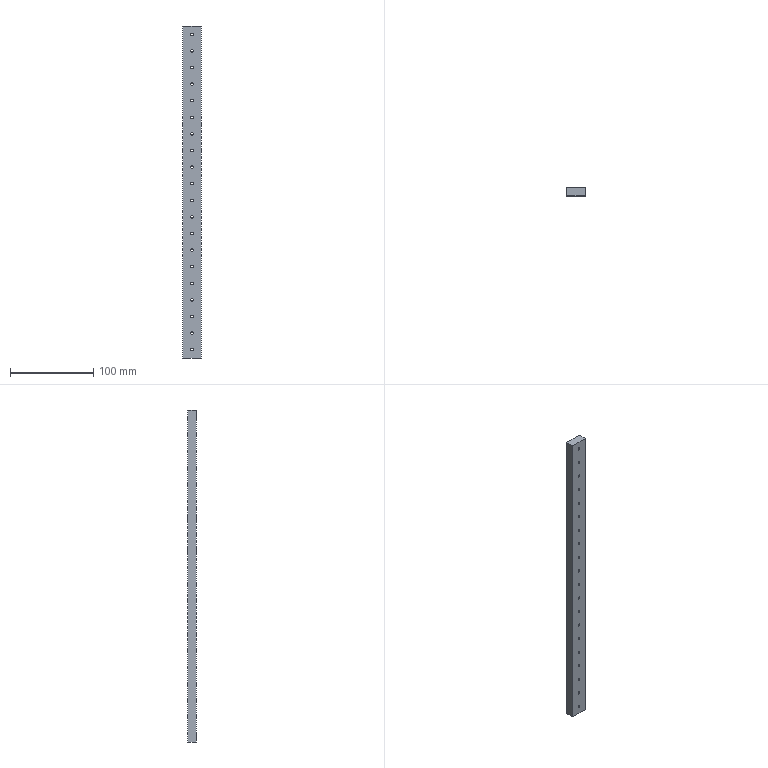Part | SolidWorks | features BaseBody 1 | 1 solid | 46 faces | box 22 x 10 x 400 mm | volume 86586 mm3 | cylinder 40 | plane 6 | commonest cylinder face diameters 3 x40
STEP:
#1=CARTESIAN_POINT('',(0.,-5.,11.5));
#2=VERTEX_POINT('',#1);
#3=CARTESIAN_POINT('',(0.,-5.,8.5));
#4=VERTEX_POINT('',#3);
#5=CARTESIAN_POINT('',(0.,-5.,10.));
#6=DIRECTION('',(0.,-1.,0.));
#7=DIRECTION('',(0.,0.,1.));
#8=AXIS2_PLACEMENT_3D('',#5,#6,#7);
#9=CIRCLE('',#8,1.5);
#10=EDGE_CURVE('',#2,#4,#9,.T.);
#11=ORIENTED_EDGE('',*,*,#10,.T.);
#12=CARTESIAN_POINT('',(0.,5.,8.5));
#13=VERTEX_POINT('',#12);
#14=CARTESIAN_POINT('',(0.,-195.,8.5));
#15=DIRECTION('',(0.,1.,0.));
#16=VECTOR('',#15,1000.);
#17=LINE('',#14,#16);
#18=EDGE_CURVE('',#4,#13,#17,.T.);
#19=ORIENTED_EDGE('',*,*,#18,.T.);
#20=CARTESIAN_POINT('',(0.,5.,11.5));
#21=VERTEX_POINT('',#20);
#22=CARTESIAN_POINT('',(0.,5.,10.));
#23=DIRECTION('',(0.,-1.,0.));
#24=DIRECTION('',(0.,0.,1.));
#25=AXIS2_PLACEMENT_3D('',#22,#23,#24);
#26=CIRCLE('',#25,1.5);
#27=EDGE_CURVE('',#21,#13,#26,.T.);
#28=ORIENTED_EDGE('',*,*,#27,.F.);
#29=CARTESIAN_POINT('',(0.,-195.,11.5));
#30=DIRECTION('',(0.,1.,0.));
#31=VECTOR('',#30,1000.);
#32=LINE('',#29,#31);
#33=EDGE_CURVE('',#2,#21,#32,.T.);
#34=ORIENTED_EDGE('',*,*,#33,.F.);
#35=EDGE_LOOP('',(#11,#19,#28,#34));
#36=FACE_OUTER_BOUND('',#35,.T.);
#37=CARTESIAN_POINT('',(0.,-195.,10.));
#38=DIRECTION('',(0.,1.,0.));
#39=DIRECTION('',(0.,0.,1.));
#40=AXIS2_PLACEMENT_3D('',#37,#38,#39);
#41=CYLINDRICAL_SURFACE('',#40,1.5);
#42=ADVANCED_FACE('',(#36),#41,.F.);
#43=CARTESIAN_POINT('',(0.,-5.,31.5));
#44=VERTEX_POINT('',#43);
#45=CARTESIAN_POINT('',(0.,-5.,28.5));
#46=VERTEX_POINT('',#45);
#47=CARTESIAN_POINT('',(0.,-5.,30.));
#48=DIRECTION('',(0.,-1.,0.));
#49=DIRECTION('',(0.,0.,1.));
#50=AXIS2_PLACEMENT_3D('',#47,#48,#49);
#51=CIRCLE('',#50,1.5);
#52=EDGE_CURVE('',#44,#46,#51,.T.);
#53=ORIENTED_EDGE('',*,*,#52,.T.);
#54=CARTESIAN_POINT('',(0.,5.,28.5));
#55=VERTEX_POINT('',#54);
#56=CARTESIAN_POINT('',(0.,-195.,28.5));
#57=DIRECTION('',(0.,1.,0.));
#58=VECTOR('',#57,1000.);
#59=LINE('',#56,#58);
#60=EDGE_CURVE('',#46,#55,#59,.T.);
#61=ORIENTED_EDGE('',*,*,#60,.T.);
#62=CARTESIAN_POINT('',(0.,5.,31.5));
#63=VERTEX_POINT('',#62);
#64=CARTESIAN_POINT('',(0.,5.,30.));
#65=DIRECTION('',(0.,-1.,0.));
#66=DIRECTION('',(0.,0.,1.));
#67=AXIS2_PLACEMENT_3D('',#64,#65,#66);
#68=CIRCLE('',#67,1.5);
#69=EDGE_CURVE('',#63,#55,#68,.T.);
#70=ORIENTED_EDGE('',*,*,#69,.F.);
#71=CARTESIAN_POINT('',(0.,-195.,31.5));
#72=DIRECTION('',(0.,1.,0.));
#73=VECTOR('',#72,1000.);
#74=LINE('',#71,#73);
#75=EDGE_CURVE('',#44,#63,#74,.T.);
#76=ORIENTED_EDGE('',*,*,#75,.F.);
#77=EDGE_LOOP('',(#53,#61,#70,#76));
#78=FACE_OUTER_BOUND('',#77,.T.);
#79=CARTESIAN_POINT('',(0.,-195.,30.));
#80=DIRECTION('',(0.,1.,0.));
#81=DIRECTION('',(0.,0.,1.));
#82=AXIS2_PLACEMENT_3D('',#79,#80,#81);
#83=CYLINDRICAL_SURFACE('',#82,1.5);
#84=ADVANCED_FACE('',(#78),#83,.F.);
#85=CARTESIAN_POINT('',(0.,-5.,51.5));
#86=VERTEX_POINT('',#85);
#87=CARTESIAN_POINT('',(0.,-5.,48.5));
#88=VERTEX_POINT('',#87);
#89=CARTESIAN_POINT('',(0.,-5.,50.));
#90=DIRECTION('',(0.,-1.,0.));
#91=DIRECTION('',(0.,0.,1.));
#92=AXIS2_PLACEMENT_3D('',#89,#90,#91);
#93=CIRCLE('',#92,1.5);
#94=EDGE_CURVE('',#86,#88,#93,.T.);
#95=ORIENTED_EDGE('',*,*,#94,.T.);
#96=CARTESIAN_POINT('',(0.,5.,48.5));
#97=VERTEX_POINT('',#96);
#98=CARTESIAN_POINT('',(0.,-195.,48.5));
#99=DIRECTION('',(0.,1.,0.));
#100=VECTOR('',#99,1000.);
#101=LINE('',#98,#100);
#102=EDGE_CURVE('',#88,#97,#101,.T.);
#103=ORIENTED_EDGE('',*,*,#102,.T.);
#104=CARTESIAN_POINT('',(0.,5.,51.5));
#105=VERTEX_POINT('',#104);
#106=CARTESIAN_POINT('',(0.,5.,50.));
#107=DIRECTION('',(0.,-1.,0.));
#108=DIRECTION('',(0.,0.,1.));
#109=AXIS2_PLACEMENT_3D('',#106,#107,#108);
#110=CIRCLE('',#109,1.5);
#111=EDGE_CURVE('',#105,#97,#110,.T.);
#112=ORIENTED_EDGE('',*,*,#111,.F.);
#113=CARTESIAN_POINT('',(0.,-195.,51.5));
#114=DIRECTION('',(0.,1.,0.));
#115=VECTOR('',#114,1000.);
#116=LINE('',#113,#115);
#117=EDGE_CURVE('',#86,#105,#116,.T.);
#118=ORIENTED_EDGE('',*,*,#117,.F.);
#119=EDGE_LOOP('',(#95,#103,#112,#118));
#120=FACE_OUTER_BOUND('',#119,.T.);
#121=CARTESIAN_POINT('',(0.,-195.,50.));
#122=DIRECTION('',(0.,1.,0.));
#123=DIRECTION('',(0.,0.,1.));
#124=AXIS2_PLACEMENT_3D('',#121,#122,#123);
#125=CYLINDRICAL_SURFACE('',#124,1.5);
#126=ADVANCED_FACE('',(#120),#125,.F.);
#127=CARTESIAN_POINT('',(0.,-5.,71.5));
#128=VERTEX_POINT('',#127);
#129=CARTESIAN_POINT('',(0.,-5.,68.5));
#130=VERTEX_POINT('',#129);
#131=CARTESIAN_POINT('',(0.,-5.,70.));
#132=DIRECTION('',(0.,-1.,0.));
#133=DIRECTION('',(0.,0.,1.));
#134=AXIS2_PLACEMENT_3D('',#131,#132,#133);
#135=CIRCLE('',#134,1.5);
#136=EDGE_CURVE('',#128,#130,#135,.T.);
#137=ORIENTED_EDGE('',*,*,#136,.T.);
#138=CARTESIAN_POINT('',(0.,5.,68.5));
#139=VERTEX_POINT('',#138);
#140=CARTESIAN_POINT('',(0.,-195.,68.5));
#141=DIRECTION('',(0.,1.,0.));
#142=VECTOR('',#141,1000.);
#143=LINE('',#140,#142);
#144=EDGE_CURVE('',#130,#139,#143,.T.);
#145=ORIENTED_EDGE('',*,*,#144,.T.);
#146=CARTESIAN_POINT('',(0.,5.,71.5));
#147=VERTEX_POINT('',#146);
#148=CARTESIAN_POINT('',(0.,5.,70.));
#149=DIRECTION('',(0.,-1.,0.));
#150=DIRECTION('',(0.,0.,1.));
#151=AXIS2_PLACEMENT_3D('',#148,#149,#150);
#152=CIRCLE('',#151,1.5);
#153=EDGE_CURVE('',#147,#139,#152,.T.);
#154=ORIENTED_EDGE('',*,*,#153,.F.);
#155=CARTESIAN_POINT('',(0.,-195.,71.5));
#156=DIRECTION('',(0.,1.,0.));
#157=VECTOR('',#156,1000.);
#158=LINE('',#155,#157);
#159=EDGE_CURVE('',#128,#147,#158,.T.);
#160=ORIENTED_EDGE('',*,*,#159,.F.);
#161=EDGE_LOOP('',(#137,#145,#154,#160));
#162=FACE_OUTER_BOUND('',#161,.T.);
#163=CARTESIAN_POINT('',(0.,-195.,70.));
#164=DIRECTION('',(0.,1.,0.));
#165=DIRECTION('',(0.,0.,1.));
#166=AXIS2_PLACEMENT_3D('',#163,#164,#165);
#167=CYLINDRICAL_SURFACE('',#166,1.5);
#168=ADVANCED_FACE('',(#162),#167,.F.);
#169=CARTESIAN_POINT('',(0.,-5.,91.5));
#170=VERTEX_POINT('',#169);
#171=CARTESIAN_POINT('',(0.,-5.,88.5));
#172=VERTEX_POINT('',#171);
#173=CARTESIAN_POINT('',(0.,-5.,90.));
#174=DIRECTION('',(0.,-1.,0.));
#175=DIRECTION('',(0.,0.,1.));
#176=AXIS2_PLACEMENT_3D('',#173,#174,#175);
#177=CIRCLE('',#176,1.5);
#178=EDGE_CURVE('',#170,#172,#177,.T.);
#179=ORIENTED_EDGE('',*,*,#178,.T.);
#180=CARTESIAN_POINT('',(0.,5.,88.5));
#181=VERTEX_POINT('',#180);
#182=CARTESIAN_POINT('',(0.,-195.,88.5));
#183=DIRECTION('',(0.,1.,0.));
#184=VECTOR('',#183,1000.);
#185=LINE('',#182,#184);
#186=EDGE_CURVE('',#172,#181,#185,.T.);
#187=ORIENTED_EDGE('',*,*,#186,.T.);
#188=CARTESIAN_POINT('',(0.,5.,91.5));
#189=VERTEX_POINT('',#188);
#190=CARTESIAN_POINT('',(0.,5.,90.));
#191=DIRECTION('',(0.,-1.,0.));
#192=DIRECTION('',(0.,0.,1.));
#193=AXIS2_PLACEMENT_3D('',#190,#191,#192);
#194=CIRCLE('',#193,1.5);
#195=EDGE_CURVE('',#189,#181,#194,.T.);
#196=ORIENTED_EDGE('',*,*,#195,.F.);
#197=CARTESIAN_POINT('',(0.,-195.,91.5));
#198=DIRECTION('',(0.,1.,0.));
#199=VECTOR('',#198,1000.);
#200=LINE('',#197,#199);
#201=EDGE_CURVE('',#170,#189,#200,.T.);
#202=ORIENTED_EDGE('',*,*,#201,.F.);
#203=EDGE_LOOP('',(#179,#187,#196,#202));
#204=FACE_OUTER_BOUND('',#203,.T.);
#205=CARTESIAN_POINT('',(0.,-195.,90.));
#206=DIRECTION('',(0.,1.,0.));
#207=DIRECTION('',(0.,0.,1.));
#208=AXIS2_PLACEMENT_3D('',#205,#206,#207);
#209=CYLINDRICAL_SURFACE('',#208,1.5);
#210=ADVANCED_FACE('',(#204),#209,.F.);
#211=CARTESIAN_POINT('',(0.,-5.,111.5));
#212=VERTEX_POINT('',#211);
#213=CARTESIAN_POINT('',(0.,-5.,108.5));
#214=VERTEX_POINT('',#213);
#215=CARTESIAN_POINT('',(0.,-5.,110.));
#216=DIRECTION('',(0.,-1.,0.));
#217=DIRECTION('',(0.,0.,1.));
#218=AXIS2_PLACEMENT_3D('',#215,#216,#217);
#219=CIRCLE('',#218,1.5);
#220=EDGE_CURVE('',#212,#214,#219,.T.);
#221=ORIENTED_EDGE('',*,*,#220,.T.);
#222=CARTESIAN_POINT('',(0.,5.,108.5));
#223=VERTEX_POINT('',#222);
#224=CARTESIAN_POINT('',(0.,-195.,108.5));
#225=DIRECTION('',(0.,1.,0.));
#226=VECTOR('',#225,1000.);
#227=LINE('',#224,#226);
#228=EDGE_CURVE('',#214,#223,#227,.T.);
#229=ORIENTED_EDGE('',*,*,#228,.T.);
#230=CARTESIAN_POINT('',(0.,5.,111.5));
#231=VERTEX_POINT('',#230);
#232=CARTESIAN_POINT('',(0.,5.,110.));
#233=DIRECTION('',(0.,-1.,0.));
#234=DIRECTION('',(0.,0.,1.));
#235=AXIS2_PLACEMENT_3D('',#232,#233,#234);
#236=CIRCLE('',#235,1.5);
#237=EDGE_CURVE('',#231,#223,#236,.T.);
#238=ORIENTED_EDGE('',*,*,#237,.F.);
#239=CARTESIAN_POINT('',(0.,-195.,111.5));
#240=DIRECTION('',(0.,1.,0.));
#241=VECTOR('',#240,1000.);
#242=LINE('',#239,#241);
#243=EDGE_CURVE('',#212,#231,#242,.T.);
#244=ORIENTED_EDGE('',*,*,#243,.F.);
#245=EDGE_LOOP('',(#221,#229,#238,#244));
#246=FACE_OUTER_BOUND('',#245,.T.);
#247=CARTESIAN_POINT('',(0.,-195.,110.));
#248=DIRECTION('',(0.,1.,0.));
#249=DIRECTION('',(0.,0.,1.));
#250=AXIS2_PLACEMENT_3D('',#247,#248,#249);
#251=CYLINDRICAL_SURFACE('',#250,1.5);
#252=ADVANCED_FACE('',(#246),#251,.F.);
#253=CARTESIAN_POINT('',(0.,-5.,131.5));
#254=VERTEX_POINT('',#253);
#255=CARTESIAN_POINT('',(0.,-5.,128.5));
#256=VERTEX_POINT('',#255);
#257=CARTESIAN_POINT('',(0.,-5.,130.));
#258=DIRECTION('',(0.,-1.,0.));
#259=DIRECTION('',(0.,0.,1.));
#260=AXIS2_PLACEMENT_3D('',#257,#258,#259);
#261=CIRCLE('',#260,1.5);
#262=EDGE_CURVE('',#254,#256,#261,.T.);
#263=ORIENTED_EDGE('',*,*,#262,.T.);
#264=CARTESIAN_POINT('',(0.,5.,128.5));
#265=VERTEX_POINT('',#264);
#266=CARTESIAN_POINT('',(0.,-195.,128.5));
#267=DIRECTION('',(0.,1.,0.));
#268=VECTOR('',#267,1000.);
#269=LINE('',#266,#268);
#270=EDGE_CURVE('',#256,#265,#269,.T.);
#271=ORIENTED_EDGE('',*,*,#270,.T.);
#272=CARTESIAN_POINT('',(0.,5.,131.5));
#273=VERTEX_POINT('',#272);
#274=CARTESIAN_POINT('',(0.,5.,130.));
#275=DIRECTION('',(0.,-1.,0.));
#276=DIRECTION('',(0.,0.,1.));
#277=AXIS2_PLACEMENT_3D('',#274,#275,#276);
#278=CIRCLE('',#277,1.5);
#279=EDGE_CURVE('',#273,#265,#278,.T.);
#280=ORIENTED_EDGE('',*,*,#279,.F.);
#281=CARTESIAN_POINT('',(0.,-195.,131.5));
#282=DIRECTION('',(0.,1.,0.));
#283=VECTOR('',#282,1000.);
#284=LINE('',#281,#283);
#285=EDGE_CURVE('',#254,#273,#284,.T.);
#286=ORIENTED_EDGE('',*,*,#285,.F.);
#287=EDGE_LOOP('',(#263,#271,#280,#286));
#288=FACE_OUTER_BOUND('',#287,.T.);
#289=CARTESIAN_POINT('',(0.,-195.,130.));
#290=DIRECTION('',(0.,1.,0.));
#291=DIRECTION('',(0.,0.,1.));
#292=AXIS2_PLACEMENT_3D('',#289,#290,#291);
#293=CYLINDRICAL_SURFACE('',#292,1.5);
#294=ADVANCED_FACE('',(#288),#293,.F.);
#295=CARTESIAN_POINT('',(0.,-5.,151.5));
#296=VERTEX_POINT('',#295);
#297=CARTESIAN_POINT('',(0.,-5.,148.5));
#298=VERTEX_POINT('',#297);
#299=CARTESIAN_POINT('',(0.,-5.,150.));
#300=DIRECTION('',(0.,-1.,0.));
#301=DIRECTION('',(0.,0.,1.));
#302=AXIS2_PLACEMENT_3D('',#299,#300,#301);
#303=CIRCLE('',#302,1.5);
#304=EDGE_CURVE('',#296,#298,#303,.T.);
#305=ORIENTED_EDGE('',*,*,#304,.T.);
#306=CARTESIAN_POINT('',(0.,5.,148.5));
#307=VERTEX_POINT('',#306);
#308=CARTESIAN_POINT('',(0.,-195.,148.5));
#309=DIRECTION('',(0.,1.,0.));
#310=VECTOR('',#309,1000.);
#311=LINE('',#308,#310);
#312=EDGE_CURVE('',#298,#307,#311,.T.);
#313=ORIENTED_EDGE('',*,*,#312,.T.);
#314=CARTESIAN_POINT('',(0.,5.,151.5));
#315=VERTEX_POINT('',#314);
#316=CARTESIAN_POINT('',(0.,5.,150.));
#317=DIRECTION('',(0.,-1.,0.));
#318=DIRECTION('',(0.,0.,1.));
#319=AXIS2_PLACEMENT_3D('',#316,#317,#318);
#320=CIRCLE('',#319,1.5);
#321=EDGE_CURVE('',#315,#307,#320,.T.);
#322=ORIENTED_EDGE('',*,*,#321,.F.);
#323=CARTESIAN_POINT('',(0.,-195.,151.5));
#324=DIRECTION('',(0.,1.,0.));
#325=VECTOR('',#324,1000.);
#326=LINE('',#323,#325);
#327=EDGE_CURVE('',#296,#315,#326,.T.);
#328=ORIENTED_EDGE('',*,*,#327,.F.);
#329=EDGE_LOOP('',(#305,#313,#322,#328));
#330=FACE_OUTER_BOUND('',#329,.T.);
#331=CARTESIAN_POINT('',(0.,-195.,150.));
#332=DIRECTION('',(0.,1.,0.));
#333=DIRECTION('',(0.,0.,1.));
#334=AXIS2_PLACEMENT_3D('',#331,#332,#333);
#335=CYLINDRICAL_SURFACE('',#334,1.5);
#336=ADVANCED_FACE('',(#330),#335,.F.);
#337=CARTESIAN_POINT('',(0.,-5.,171.5));
#338=VERTEX_POINT('',#337);
#339=CARTESIAN_POINT('',(0.,-5.,168.5));
#340=VERTEX_POINT('',#339);
#341=CARTESIAN_POINT('',(0.,-5.,170.));
#342=DIRECTION('',(0.,-1.,0.));
#343=DIRECTION('',(0.,0.,1.));
#344=AXIS2_PLACEMENT_3D('',#341,#342,#343);
#345=CIRCLE('',#344,1.5);
#346=EDGE_CURVE('',#338,#340,#345,.T.);
#347=ORIENTED_EDGE('',*,*,#346,.T.);
#348=CARTESIAN_POINT('',(0.,5.,168.5));
#349=VERTEX_POINT('',#348);
#350=CARTESIAN_POINT('',(0.,-195.,168.5));
#351=DIRECTION('',(0.,1.,0.));
#352=VECTOR('',#351,1000.);
#353=LINE('',#350,#352);
#354=EDGE_CURVE('',#340,#349,#353,.T.);
#355=ORIENTED_EDGE('',*,*,#354,.T.);
#356=CARTESIAN_POINT('',(0.,5.,171.5));
#357=VERTEX_POINT('',#356);
#358=CARTESIAN_POINT('',(0.,5.,170.));
#359=DIRECTION('',(0.,-1.,0.));
#360=DIRECTION('',(0.,0.,1.));
#361=AXIS2_PLACEMENT_3D('',#358,#359,#360);
#362=CIRCLE('',#361,1.5);
#363=EDGE_CURVE('',#357,#349,#362,.T.);
#364=ORIENTED_EDGE('',*,*,#363,.F.);
#365=CARTESIAN_POINT('',(0.,-195.,171.5));
#366=DIRECTION('',(0.,1.,0.));
#367=VECTOR('',#366,1000.);
#368=LINE('',#365,#367);
#369=EDGE_CURVE('',#338,#357,#368,.T.);
#370=ORIENTED_EDGE('',*,*,#369,.F.);
#371=EDGE_LOOP('',(#347,#355,#364,#370));
#372=FACE_OUTER_BOUND('',#371,.T.);
#373=CARTESIAN_POINT('',(0.,-195.,170.));
#374=DIRECTION('',(0.,1.,0.));
#375=DIRECTION('',(0.,0.,1.));
#376=AXIS2_PLACEMENT_3D('',#373,#374,#375);
#377=CYLINDRICAL_SURFACE('',#376,1.5);
#378=ADVANCED_FACE('',(#372),#377,.F.);
#379=CARTESIAN_POINT('',(0.,-5.,191.5));
#380=VERTEX_POINT('',#379);
#381=CARTESIAN_POINT('',(0.,-5.,188.5));
#382=VERTEX_POINT('',#381);
#383=CARTESIAN_POINT('',(0.,-5.,190.));
#384=DIRECTION('',(0.,-1.,0.));
#385=DIRECTION('',(0.,0.,1.));
#386=AXIS2_PLACEMENT_3D('',#383,#384,#385);
#387=CIRCLE('',#386,1.5);
#388=EDGE_CURVE('',#380,#382,#387,.T.);
#389=ORIENTED_EDGE('',*,*,#388,.T.);
#390=CARTESIAN_POINT('',(0.,5.,188.5));
#391=VERTEX_POINT('',#390);
#392=CARTESIAN_POINT('',(0.,-195.,188.5));
#393=DIRECTION('',(0.,1.,0.));
#394=VECTOR('',#393,1000.);
#395=LINE('',#392,#394);
#396=EDGE_CURVE('',#382,#391,#395,.T.);
#397=ORIENTED_EDGE('',*,*,#396,.T.);
#398=CARTESIAN_POINT('',(0.,5.,191.5));
#399=VERTEX_POINT('',#398);
#400=CARTESIAN_POINT('',(0.,5.,190.));
#401=DIRECTION('',(0.,-1.,0.));
#402=DIRECTION('',(0.,0.,1.));
#403=AXIS2_PLACEMENT_3D('',#400,#401,#402);
#404=CIRCLE('',#403,1.5);
#405=EDGE_CURVE('',#399,#391,#404,.T.);
#406=ORIENTED_EDGE('',*,*,#405,.F.);
#407=CARTESIAN_POINT('',(0.,-195.,191.5));
#408=DIRECTION('',(0.,1.,0.));
#409=VECTOR('',#408,1000.);
#410=LINE('',#407,#409);
#411=EDGE_CURVE('',#380,#399,#410,.T.);
#412=ORIENTED_EDGE('',*,*,#411,.F.);
#413=EDGE_LOOP('',(#389,#397,#406,#412));
#414=FACE_OUTER_BOUND('',#413,.T.);
#415=CARTESIAN_POINT('',(0.,-195.,190.));
#416=DIRECTION('',(0.,1.,0.));
#417=DIRECTION('',(0.,0.,1.));
#418=AXIS2_PLACEMENT_3D('',#415,#416,#417);
#419=CYLINDRICAL_SURFACE('',#418,1.5);
#420=ADVANCED_FACE('',(#414),#419,.F.);
#421=CARTESIAN_POINT('',(0.,-5.,211.5));
#422=VERTEX_POINT('',#421);
#423=CARTESIAN_POINT('',(0.,-5.,208.5));
#424=VERTEX_POINT('',#423);
#425=CARTESIAN_POINT('',(0.,-5.,210.));
#426=DIRECTION('',(0.,-1.,0.));
#427=DIRECTION('',(0.,0.,1.));
#428=AXIS2_PLACEMENT_3D('',#425,#426,#427);
#429=CIRCLE('',#428,1.5);
#430=EDGE_CURVE('',#422,#424,#429,.T.);
#431=ORIENTED_EDGE('',*,*,#430,.T.);
#432=CARTESIAN_POINT('',(0.,5.,208.5));
#433=VERTEX_POINT('',#432);
#434=CARTESIAN_POINT('',(0.,-195.,208.5));
#435=DIRECTION('',(0.,1.,0.));
#436=VECTOR('',#435,1000.);
#437=LINE('',#434,#436);
#438=EDGE_CURVE('',#424,#433,#437,.T.);
#439=ORIENTED_EDGE('',*,*,#438,.T.);
#440=CARTESIAN_POINT('',(0.,5.,211.5));
#441=VERTEX_POINT('',#440);
#442=CARTESIAN_POINT('',(0.,5.,210.));
#443=DIRECTION('',(0.,-1.,0.));
#444=DIRECTION('',(0.,0.,1.));
#445=AXIS2_PLACEMENT_3D('',#442,#443,#444);
#446=CIRCLE('',#445,1.5);
#447=EDGE_CURVE('',#441,#433,#446,.T.);
#448=ORIENTED_EDGE('',*,*,#447,.F.);
#449=CARTESIAN_POINT('',(0.,-195.,211.5));
#450=DIRECTION('',(0.,1.,0.));
#451=VECTOR('',#450,1000.);
#452=LINE('',#449,#451);
#453=EDGE_CURVE('',#422,#441,#452,.T.);
#454=ORIENTED_EDGE('',*,*,#453,.F.);
#455=EDGE_LOOP('',(#431,#439,#448,#454));
#456=FACE_OUTER_BOUND('',#455,.T.);
#457=CARTESIAN_POINT('',(0.,-195.,210.));
#458=DIRECTION('',(0.,1.,0.));
#459=DIRECTION('',(0.,0.,1.));
#460=AXIS2_PLACEMENT_3D('',#457,#458,#459);
#461=CYLINDRICAL_SURFACE('',#460,1.5);
#462=ADVANCED_FACE('',(#456),#461,.F.);
#463=CARTESIAN_POINT('',(0.,-5.,231.5));
#464=VERTEX_POINT('',#463);
#465=CARTESIAN_POINT('',(0.,-5.,228.5));
#466=VERTEX_POINT('',#465);
#467=CARTESIAN_POINT('',(0.,-5.,230.));
#468=DIRECTION('',(0.,-1.,0.));
#469=DIRECTION('',(0.,0.,1.));
#470=AXIS2_PLACEMENT_3D('',#467,#468,#469);
#471=CIRCLE('',#470,1.5);
#472=EDGE_CURVE('',#464,#466,#471,.T.);
#473=ORIENTED_EDGE('',*,*,#472,.T.);
#474=CARTESIAN_POINT('',(0.,5.,228.5));
#475=VERTEX_POINT('',#474);
#476=CARTESIAN_POINT('',(0.,-195.,228.5));
#477=DIRECTION('',(0.,1.,0.));
#478=VECTOR('',#477,1000.);
#479=LINE('',#476,#478);
#480=EDGE_CURVE('',#466,#475,#479,.T.);
#481=ORIENTED_EDGE('',*,*,#480,.T.);
#482=CARTESIAN_POINT('',(0.,5.,231.5));
#483=VERTEX_POINT('',#482);
#484=CARTESIAN_POINT('',(0.,5.,230.));
#485=DIRECTION('',(0.,-1.,0.));
#486=DIRECTION('',(0.,0.,1.));
#487=AXIS2_PLACEMENT_3D('',#484,#485,#486);
#488=CIRCLE('',#487,1.5);
#489=EDGE_CURVE('',#483,#475,#488,.T.);
#490=ORIENTED_EDGE('',*,*,#489,.F.);
#491=CARTESIAN_POINT('',(0.,-195.,231.5));
#492=DIRECTION('',(0.,1.,0.));
#493=VECTOR('',#492,1000.);
#494=LINE('',#491,#493);
#495=EDGE_CURVE('',#464,#483,#494,.T.);
#496=ORIENTED_EDGE('',*,*,#495,.F.);
#497=EDGE_LOOP('',(#473,#481,#490,#496));
#498=FACE_OUTER_BOUND('',#497,.T.);
#499=CARTESIAN_POINT('',(0.,-195.,230.));
#500=DIRECTION('',(0.,1.,0.));
#501=DIRECTION('',(0.,0.,1.));
#502=AXIS2_PLACEMENT_3D('',#499,#500,#501);
#503=CYLINDRICAL_SURFACE('',#502,1.5);
#504=ADVANCED_FACE('',(#498),#503,.F.);
#505=CARTESIAN_POINT('',(0.,-5.,251.5));
#506=VERTEX_POINT('',#505);
#507=CARTESIAN_POINT('',(0.,-5.,248.5));
#508=VERTEX_POINT('',#507);
#509=CARTESIAN_POINT('',(0.,-5.,250.));
#510=DIRECTION('',(0.,-1.,0.));
#511=DIRECTION('',(0.,0.,1.));
#512=AXIS2_PLACEMENT_3D('',#509,#510,#511);
#513=CIRCLE('',#512,1.5);
#514=EDGE_CURVE('',#506,#508,#513,.T.);
#515=ORIENTED_EDGE('',*,*,#514,.T.);
#516=CARTESIAN_POINT('',(0.,5.,248.5));
#517=VERTEX_POINT('',#516);
#518=CARTESIAN_POINT('',(0.,-195.,248.5));
#519=DIRECTION('',(0.,1.,0.));
#520=VECTOR('',#519,1000.);
#521=LINE('',#518,#520);
#522=EDGE_CURVE('',#508,#517,#521,.T.);
#523=ORIENTED_EDGE('',*,*,#522,.T.);
#524=CARTESIAN_POINT('',(0.,5.,251.5));
#525=VERTEX_POINT('',#524);
#526=CARTESIAN_POINT('',(0.,5.,250.));
#527=DIRECTION('',(0.,-1.,0.));
#528=DIRECTION('',(0.,0.,1.));
#529=AXIS2_PLACEMENT_3D('',#526,#527,#528);
#530=CIRCLE('',#529,1.5);
#531=EDGE_CURVE('',#525,#517,#530,.T.);
#532=ORIENTED_EDGE('',*,*,#531,.F.);
#533=CARTESIAN_POINT('',(0.,-195.,251.5));
#534=DIRECTION('',(0.,1.,0.));
#535=VECTOR('',#534,1000.);
#536=LINE('',#533,#535);
#537=EDGE_CURVE('',#506,#525,#536,.T.);
#538=ORIENTED_EDGE('',*,*,#537,.F.);
#539=EDGE_LOOP('',(#515,#523,#532,#538));
#540=FACE_OUTER_BOUND('',#539,.T.);
#541=CARTESIAN_POINT('',(0.,-195.,250.));
#542=DIRECTION('',(0.,1.,0.));
#543=DIRECTION('',(0.,0.,1.));
#544=AXIS2_PLACEMENT_3D('',#541,#542,#543);
#545=CYLINDRICAL_SURFACE('',#544,1.5);
#546=ADVANCED_FACE('',(#540),#545,.F.);
#547=CARTESIAN_POINT('',(0.,-5.,271.5));
#548=VERTEX_POINT('',#547);
#549=CARTESIAN_POINT('',(0.,-5.,268.5));
#550=VERTEX_POINT('',#549);
#551=CARTESIAN_POINT('',(0.,-5.,270.));
#552=DIRECTION('',(0.,-1.,0.));
#553=DIRECTION('',(0.,0.,1.));
#554=AXIS2_PLACEMENT_3D('',#551,#552,#553);
#555=CIRCLE('',#554,1.5);
#556=EDGE_CURVE('',#548,#550,#555,.T.);
#557=ORIENTED_EDGE('',*,*,#556,.T.);
#558=CARTESIAN_POINT('',(0.,5.,268.5));
#559=VERTEX_POINT('',#558);
#560=CARTESIAN_POINT('',(0.,-195.,268.5));
#561=DIRECTION('',(0.,1.,0.));
#562=VECTOR('',#561,1000.);
#563=LINE('',#560,#562);
#564=EDGE_CURVE('',#550,#559,#563,.T.);
#565=ORIENTED_EDGE('',*,*,#564,.T.);
#566=CARTESIAN_POINT('',(0.,5.,271.5));
#567=VERTEX_POINT('',#566);
#568=CARTESIAN_POINT('',(0.,5.,270.));
#569=DIRECTION('',(0.,-1.,0.));
#570=DIRECTION('',(0.,0.,1.));
#571=AXIS2_PLACEMENT_3D('',#568,#569,#570);
#572=CIRCLE('',#571,1.5);
#573=EDGE_CURVE('',#567,#559,#572,.T.);
#574=ORIENTED_EDGE('',*,*,#573,.F.);
#575=CARTESIAN_POINT('',(0.,-195.,271.5));
#576=DIRECTION('',(0.,1.,0.));
#577=VECTOR('',#576,1000.);
#578=LINE('',#575,#577);
#579=EDGE_CURVE('',#548,#567,#578,.T.);
#580=ORIENTED_EDGE('',*,*,#579,.F.);
#581=EDGE_LOOP('',(#557,#565,#574,#580));
#582=FACE_OUTER_BOUND('',#581,.T.);
#583=CARTESIAN_POINT('',(0.,-195.,270.));
#584=DIRECTION('',(0.,1.,0.));
#585=DIRECTION('',(0.,0.,1.));
#586=AXIS2_PLACEMENT_3D('',#583,#584,#585);
#587=CYLINDRICAL_SURFACE('',#586,1.5);
#588=ADVANCED_FACE('',(#582),#587,.F.);
#589=CARTESIAN_POINT('',(0.,-5.,291.5));
#590=VERTEX_POINT('',#589);
#591=CARTESIAN_POINT('',(0.,-5.,288.5));
#592=VERTEX_POINT('',#591);
#593=CARTESIAN_POINT('',(0.,-5.,290.));
#594=DIRECTION('',(0.,-1.,0.));
#595=DIRECTION('',(0.,0.,1.));
#596=AXIS2_PLACEMENT_3D('',#593,#594,#595);
#597=CIRCLE('',#596,1.5);
#598=EDGE_CURVE('',#590,#592,#597,.T.);
#599=ORIENTED_EDGE('',*,*,#598,.T.);
#600=CARTESIAN_POINT('',(0.,5.,288.5));
#601=VERTEX_POINT('',#600);
#602=CARTESIAN_POINT('',(0.,-195.,288.5));
#603=DIRECTION('',(0.,1.,0.));
#604=VECTOR('',#603,1000.);
#605=LINE('',#602,#604);
#606=EDGE_CURVE('',#592,#601,#605,.T.);
#607=ORIENTED_EDGE('',*,*,#606,.T.);
#608=CARTESIAN_POINT('',(0.,5.,291.5));
#609=VERTEX_POINT('',#608);
#610=CARTESIAN_POINT('',(0.,5.,290.));
#611=DIRECTION('',(0.,-1.,0.));
#612=DIRECTION('',(0.,0.,1.));
#613=AXIS2_PLACEMENT_3D('',#610,#611,#612);
#614=CIRCLE('',#613,1.5);
#615=EDGE_CURVE('',#609,#601,#614,.T.);
#616=ORIENTED_EDGE('',*,*,#615,.F.);
#617=CARTESIAN_POINT('',(0.,-195.,291.5));
#618=DIRECTION('',(0.,1.,0.));
#619=VECTOR('',#618,1000.);
#620=LINE('',#617,#619);
#621=EDGE_CURVE('',#590,#609,#620,.T.);
#622=ORIENTED_EDGE('',*,*,#621,.F.);
#623=EDGE_LOOP('',(#599,#607,#616,#622));
#624=FACE_OUTER_BOUND('',#623,.T.);
#625=CARTESIAN_POINT('',(0.,-195.,290.));
#626=DIRECTION('',(0.,1.,0.));
#627=DIRECTION('',(0.,0.,1.));
#628=AXIS2_PLACEMENT_3D('',#625,#626,#627);
#629=CYLINDRICAL_SURFACE('',#628,1.5);
#630=ADVANCED_FACE('',(#624),#629,.F.);
#631=CARTESIAN_POINT('',(0.,-5.,311.5));
#632=VERTEX_POINT('',#631);
#633=CARTESIAN_POINT('',(0.,-5.,308.5));
#634=VERTEX_POINT('',#633);
#635=CARTESIAN_POINT('',(0.,-5.,310.));
#636=DIRECTION('',(0.,-1.,0.));
#637=DIRECTION('',(0.,0.,1.));
#638=AXIS2_PLACEMENT_3D('',#635,#636,#637);
#639=CIRCLE('',#638,1.5);
#640=EDGE_CURVE('',#632,#634,#639,.T.);
#641=ORIENTED_EDGE('',*,*,#640,.T.);
#642=CARTESIAN_POINT('',(0.,5.,308.5));
#643=VERTEX_POINT('',#642);
#644=CARTESIAN_POINT('',(0.,-195.,308.5));
#645=DIRECTION('',(0.,1.,0.));
#646=VECTOR('',#645,1000.);
#647=LINE('',#644,#646);
#648=EDGE_CURVE('',#634,#643,#647,.T.);
#649=ORIENTED_EDGE('',*,*,#648,.T.);
#650=CARTESIAN_POINT('',(0.,5.,311.5));
#651=VERTEX_POINT('',#650);
#652=CARTESIAN_POINT('',(0.,5.,310.));
#653=DIRECTION('',(0.,-1.,0.));
#654=DIRECTION('',(0.,0.,1.));
#655=AXIS2_PLACEMENT_3D('',#652,#653,#654);
#656=CIRCLE('',#655,1.5);
#657=EDGE_CURVE('',#651,#643,#656,.T.);
#658=ORIENTED_EDGE('',*,*,#657,.F.);
#659=CARTESIAN_POINT('',(0.,-195.,311.5));
#660=DIRECTION('',(0.,1.,0.));
#661=VECTOR('',#660,1000.);
#662=LINE('',#659,#661);
#663=EDGE_CURVE('',#632,#651,#662,.T.);
#664=ORIENTED_EDGE('',*,*,#663,.F.);
#665=EDGE_LOOP('',(#641,#649,#658,#664));
#666=FACE_OUTER_BOUND('',#665,.T.);
#667=CARTESIAN_POINT('',(0.,-195.,310.));
#668=DIRECTION('',(0.,1.,0.));
#669=DIRECTION('',(0.,0.,1.));
#670=AXIS2_PLACEMENT_3D('',#667,#668,#669);
#671=CYLINDRICAL_SURFACE('',#670,1.5);
#672=ADVANCED_FACE('',(#666),#671,.F.);
#673=CARTESIAN_POINT('',(0.,-5.,331.5));
#674=VERTEX_POINT('',#673);
#675=CARTESIAN_POINT('',(0.,-5.,328.5));
#676=VERTEX_POINT('',#675);
#677=CARTESIAN_POINT('',(0.,-5.,330.));
#678=DIRECTION('',(0.,-1.,0.));
#679=DIRECTION('',(0.,0.,1.));
#680=AXIS2_PLACEMENT_3D('',#677,#678,#679);
#681=CIRCLE('',#680,1.5);
#682=EDGE_CURVE('',#674,#676,#681,.T.);
#683=ORIENTED_EDGE('',*,*,#682,.T.);
#684=CARTESIAN_POINT('',(0.,5.,328.5));
#685=VERTEX_POINT('',#684);
#686=CARTESIAN_POINT('',(0.,-195.,328.5));
#687=DIRECTION('',(0.,1.,0.));
#688=VECTOR('',#687,1000.);
#689=LINE('',#686,#688);
#690=EDGE_CURVE('',#676,#685,#689,.T.);
#691=ORIENTED_EDGE('',*,*,#690,.T.);
#692=CARTESIAN_POINT('',(0.,5.,331.5));
#693=VERTEX_POINT('',#692);
#694=CARTESIAN_POINT('',(0.,5.,330.));
#695=DIRECTION('',(0.,-1.,0.));
#696=DIRECTION('',(0.,0.,1.));
#697=AXIS2_PLACEMENT_3D('',#694,#695,#696);
#698=CIRCLE('',#697,1.5);
#699=EDGE_CURVE('',#693,#685,#698,.T.);
#700=ORIENTED_EDGE('',*,*,#699,.F.);
#701=CARTESIAN_POINT('',(0.,-195.,331.5));
#702=DIRECTION('',(0.,1.,0.));
#703=VECTOR('',#702,1000.);
#704=LINE('',#701,#703);
#705=EDGE_CURVE('',#674,#693,#704,.T.);
#706=ORIENTED_EDGE('',*,*,#705,.F.);
#707=EDGE_LOOP('',(#683,#691,#700,#706));
#708=FACE_OUTER_BOUND('',#707,.T.);
#709=CARTESIAN_POINT('',(0.,-195.,330.));
#710=DIRECTION('',(0.,1.,0.));
#711=DIRECTION('',(0.,0.,1.));
#712=AXIS2_PLACEMENT_3D('',#709,#710,#711);
#713=CYLINDRICAL_SURFACE('',#712,1.5);
#714=ADVANCED_FACE('',(#708),#713,.F.);
#715=CARTESIAN_POINT('',(0.,-5.,351.5));
#716=VERTEX_POINT('',#715);
#717=CARTESIAN_POINT('',(0.,-5.,348.5));
#718=VERTEX_POINT('',#717);
#719=CARTESIAN_POINT('',(0.,-5.,350.));
#720=DIRECTION('',(0.,-1.,0.));
#721=DIRECTION('',(0.,0.,1.));
#722=AXIS2_PLACEMENT_3D('',#719,#720,#721);
#723=CIRCLE('',#722,1.5);
#724=EDGE_CURVE('',#716,#718,#723,.T.);
#725=ORIENTED_EDGE('',*,*,#724,.T.);
#726=CARTESIAN_POINT('',(0.,5.,348.5));
#727=VERTEX_POINT('',#726);
#728=CARTESIAN_POINT('',(0.,-195.,348.5));
#729=DIRECTION('',(0.,1.,0.));
#730=VECTOR('',#729,1000.);
#731=LINE('',#728,#730);
#732=EDGE_CURVE('',#718,#727,#731,.T.);
#733=ORIENTED_EDGE('',*,*,#732,.T.);
#734=CARTESIAN_POINT('',(0.,5.,351.5));
#735=VERTEX_POINT('',#734);
#736=CARTESIAN_POINT('',(0.,5.,350.));
#737=DIRECTION('',(0.,-1.,0.));
#738=DIRECTION('',(0.,0.,1.));
#739=AXIS2_PLACEMENT_3D('',#736,#737,#738);
#740=CIRCLE('',#739,1.5);
#741=EDGE_CURVE('',#735,#727,#740,.T.);
#742=ORIENTED_EDGE('',*,*,#741,.F.);
#743=CARTESIAN_POINT('',(0.,-195.,351.5));
#744=DIRECTION('',(0.,1.,0.));
#745=VECTOR('',#744,1000.);
#746=LINE('',#743,#745);
#747=EDGE_CURVE('',#716,#735,#746,.T.);
#748=ORIENTED_EDGE('',*,*,#747,.F.);
#749=EDGE_LOOP('',(#725,#733,#742,#748));
#750=FACE_OUTER_BOUND('',#749,.T.);
#751=CARTESIAN_POINT('',(0.,-195.,350.));
#752=DIRECTION('',(0.,1.,0.));
#753=DIRECTION('',(0.,0.,1.));
#754=AXIS2_PLACEMENT_3D('',#751,#752,#753);
#755=CYLINDRICAL_SURFACE('',#754,1.5);
#756=ADVANCED_FACE('',(#750),#755,.F.);
#757=CARTESIAN_POINT('',(0.,-5.,371.5));
#758=VERTEX_POINT('',#757);
#759=CARTESIAN_POINT('',(0.,-5.,368.5));
#760=VERTEX_POINT('',#759);
#761=CARTESIAN_POINT('',(0.,-5.,370.));
#762=DIRECTION('',(0.,-1.,0.));
#763=DIRECTION('',(0.,0.,1.));
#764=AXIS2_PLACEMENT_3D('',#761,#762,#763);
#765=CIRCLE('',#764,1.5);
#766=EDGE_CURVE('',#758,#760,#765,.T.);
#767=ORIENTED_EDGE('',*,*,#766,.T.);
#768=CARTESIAN_POINT('',(0.,5.,368.5));
#769=VERTEX_POINT('',#768);
#770=CARTESIAN_POINT('',(0.,-195.,368.5));
#771=DIRECTION('',(0.,1.,0.));
#772=VECTOR('',#771,1000.);
#773=LINE('',#770,#772);
#774=EDGE_CURVE('',#760,#769,#773,.T.);
#775=ORIENTED_EDGE('',*,*,#774,.T.);
#776=CARTESIAN_POINT('',(0.,5.,371.5));
#777=VERTEX_POINT('',#776);
#778=CARTESIAN_POINT('',(0.,5.,370.));
#779=DIRECTION('',(0.,-1.,0.));
#780=DIRECTION('',(0.,0.,1.));
#781=AXIS2_PLACEMENT_3D('',#778,#779,#780);
#782=CIRCLE('',#781,1.5);
#783=EDGE_CURVE('',#777,#769,#782,.T.);
#784=ORIENTED_EDGE('',*,*,#783,.F.);
#785=CARTESIAN_POINT('',(0.,-195.,371.5));
#786=DIRECTION('',(0.,1.,0.));
#787=VECTOR('',#786,1000.);
#788=LINE('',#785,#787);
#789=EDGE_CURVE('',#758,#777,#788,.T.);
#790=ORIENTED_EDGE('',*,*,#789,.F.);
#791=EDGE_LOOP('',(#767,#775,#784,#790));
#792=FACE_OUTER_BOUND('',#791,.T.);
#793=CARTESIAN_POINT('',(0.,-195.,370.));
#794=DIRECTION('',(0.,1.,0.));
#795=DIRECTION('',(0.,0.,1.));
#796=AXIS2_PLACEMENT_3D('',#793,#794,#795);
#797=CYLINDRICAL_SURFACE('',#796,1.5);
#798=ADVANCED_FACE('',(#792),#797,.F.);
#799=CARTESIAN_POINT('',(0.,-5.,391.5));
#800=VERTEX_POINT('',#799);
#801=CARTESIAN_POINT('',(0.,-5.,388.5));
#802=VERTEX_POINT('',#801);
#803=CARTESIAN_POINT('',(0.,-5.,390.));
#804=DIRECTION('',(0.,-1.,0.));
#805=DIRECTION('',(0.,0.,1.));
#806=AXIS2_PLACEMENT_3D('',#803,#804,#805);
#807=CIRCLE('',#806,1.5);
#808=EDGE_CURVE('',#800,#802,#807,.T.);
#809=ORIENTED_EDGE('',*,*,#808,.T.);
#810=CARTESIAN_POINT('',(0.,5.,388.5));
#811=VERTEX_POINT('',#810);
#812=CARTESIAN_POINT('',(0.,-195.,388.5));
#813=DIRECTION('',(0.,1.,0.));
#814=VECTOR('',#813,1000.);
#815=LINE('',#812,#814);
#816=EDGE_CURVE('',#802,#811,#815,.T.);
#817=ORIENTED_EDGE('',*,*,#816,.T.);
#818=CARTESIAN_POINT('',(0.,5.,391.5));
#819=VERTEX_POINT('',#818);
#820=CARTESIAN_POINT('',(0.,5.,390.));
#821=DIRECTION('',(0.,-1.,0.));
#822=DIRECTION('',(0.,0.,1.));
#823=AXIS2_PLACEMENT_3D('',#820,#821,#822);
#824=CIRCLE('',#823,1.5);
#825=EDGE_CURVE('',#819,#811,#824,.T.);
#826=ORIENTED_EDGE('',*,*,#825,.F.);
#827=CARTESIAN_POINT('',(0.,-195.,391.5));
#828=DIRECTION('',(0.,1.,0.));
#829=VECTOR('',#828,1000.);
#830=LINE('',#827,#829);
#831=EDGE_CURVE('',#800,#819,#830,.T.);
#832=ORIENTED_EDGE('',*,*,#831,.F.);
#833=EDGE_LOOP('',(#809,#817,#826,#832));
#834=FACE_OUTER_BOUND('',#833,.T.);
#835=CARTESIAN_POINT('',(0.,-195.,390.));
#836=DIRECTION('',(0.,1.,0.));
#837=DIRECTION('',(0.,0.,1.));
#838=AXIS2_PLACEMENT_3D('',#835,#836,#837);
#839=CYLINDRICAL_SURFACE('',#838,1.5);
#840=ADVANCED_FACE('',(#834),#839,.F.);
#841=CARTESIAN_POINT('',(11.,-5.,400.));
#842=VERTEX_POINT('',#841);
#843=CARTESIAN_POINT('',(11.,-5.,0.));
#844=VERTEX_POINT('',#843);
#845=CARTESIAN_POINT('',(11.,-5.,400.));
#846=DIRECTION('',(0.,0.,-1.));
#847=VECTOR('',#846,1000.);
#848=LINE('',#845,#847);
#849=EDGE_CURVE('',#842,#844,#848,.T.);
#850=ORIENTED_EDGE('',*,*,#849,.F.);
#851=CARTESIAN_POINT('',(-11.,-5.,400.));
#852=VERTEX_POINT('',#851);
#853=CARTESIAN_POINT('',(-11.,-5.,400.));
#854=DIRECTION('',(1.,0.,0.));
#855=VECTOR('',#854,1000.);
#856=LINE('',#853,#855);
#857=EDGE_CURVE('',#852,#842,#856,.T.);
#858=ORIENTED_EDGE('',*,*,#857,.F.);
#859=CARTESIAN_POINT('',(-11.,-5.,0.));
#860=VERTEX_POINT('',#859);
#861=CARTESIAN_POINT('',(-11.,-5.,400.));
#862=DIRECTION('',(0.,0.,1.));
#863=VECTOR('',#862,1000.);
#864=LINE('',#861,#863);
#865=EDGE_CURVE('',#860,#852,#864,.T.);
#866=ORIENTED_EDGE('',*,*,#865,.F.);
#867=CARTESIAN_POINT('',(-11.,-5.,0.));
#868=DIRECTION('',(-1.,0.,0.));
#869=VECTOR('',#868,1000.);
#870=LINE('',#867,#869);
#871=EDGE_CURVE('',#844,#860,#870,.T.);
#872=ORIENTED_EDGE('',*,*,#871,.F.);
#873=EDGE_LOOP('',(#850,#858,#866,#872));
#874=FACE_OUTER_BOUND('',#873,.T.);
#875=ORIENTED_EDGE('',*,*,#10,.F.);
#876=CARTESIAN_POINT('',(0.,-5.,10.));
#877=DIRECTION('',(0.,-1.,0.));
#878=DIRECTION('',(0.,0.,1.));
#879=AXIS2_PLACEMENT_3D('',#876,#877,#878);
#880=CIRCLE('',#879,1.5);
#881=EDGE_CURVE('',#4,#2,#880,.T.);
#882=ORIENTED_EDGE('',*,*,#881,.F.);
#883=EDGE_LOOP('',(#875,#882));
#884=FACE_BOUND('',#883,.T.);
#885=ORIENTED_EDGE('',*,*,#52,.F.);
#886=CARTESIAN_POINT('',(0.,-5.,30.));
#887=DIRECTION('',(0.,-1.,0.));
#888=DIRECTION('',(0.,0.,1.));
#889=AXIS2_PLACEMENT_3D('',#886,#887,#888);
#890=CIRCLE('',#889,1.5);
#891=EDGE_CURVE('',#46,#44,#890,.T.);
#892=ORIENTED_EDGE('',*,*,#891,.F.);
#893=EDGE_LOOP('',(#885,#892));
#894=FACE_BOUND('',#893,.T.);
#895=ORIENTED_EDGE('',*,*,#94,.F.);
#896=CARTESIAN_POINT('',(0.,-5.,50.));
#897=DIRECTION('',(0.,-1.,0.));
#898=DIRECTION('',(0.,0.,1.));
#899=AXIS2_PLACEMENT_3D('',#896,#897,#898);
#900=CIRCLE('',#899,1.5);
#901=EDGE_CURVE('',#88,#86,#900,.T.);
#902=ORIENTED_EDGE('',*,*,#901,.F.);
#903=EDGE_LOOP('',(#895,#902));
#904=FACE_BOUND('',#903,.T.);
#905=ORIENTED_EDGE('',*,*,#136,.F.);
#906=CARTESIAN_POINT('',(0.,-5.,70.));
#907=DIRECTION('',(0.,-1.,0.));
#908=DIRECTION('',(0.,0.,1.));
#909=AXIS2_PLACEMENT_3D('',#906,#907,#908);
#910=CIRCLE('',#909,1.5);
#911=EDGE_CURVE('',#130,#128,#910,.T.);
#912=ORIENTED_EDGE('',*,*,#911,.F.);
#913=EDGE_LOOP('',(#905,#912));
#914=FACE_BOUND('',#913,.T.);
#915=ORIENTED_EDGE('',*,*,#178,.F.);
#916=CARTESIAN_POINT('',(0.,-5.,90.));
#917=DIRECTION('',(0.,-1.,0.));
#918=DIRECTION('',(0.,0.,1.));
#919=AXIS2_PLACEMENT_3D('',#916,#917,#918);
#920=CIRCLE('',#919,1.5);
#921=EDGE_CURVE('',#172,#170,#920,.T.);
#922=ORIENTED_EDGE('',*,*,#921,.F.);
#923=EDGE_LOOP('',(#915,#922));
#924=FACE_BOUND('',#923,.T.);
#925=ORIENTED_EDGE('',*,*,#220,.F.);
#926=CARTESIAN_POINT('',(0.,-5.,110.));
#927=DIRECTION('',(0.,-1.,0.));
#928=DIRECTION('',(0.,0.,1.));
#929=AXIS2_PLACEMENT_3D('',#926,#927,#928);
#930=CIRCLE('',#929,1.5);
#931=EDGE_CURVE('',#214,#212,#930,.T.);
#932=ORIENTED_EDGE('',*,*,#931,.F.);
#933=EDGE_LOOP('',(#925,#932));
#934=FACE_BOUND('',#933,.T.);
#935=ORIENTED_EDGE('',*,*,#262,.F.);
#936=CARTESIAN_POINT('',(0.,-5.,130.));
#937=DIRECTION('',(0.,-1.,0.));
#938=DIRECTION('',(0.,0.,1.));
#939=AXIS2_PLACEMENT_3D('',#936,#937,#938);
#940=CIRCLE('',#939,1.5);
#941=EDGE_CURVE('',#256,#254,#940,.T.);
#942=ORIENTED_EDGE('',*,*,#941,.F.);
#943=EDGE_LOOP('',(#935,#942));
#944=FACE_BOUND('',#943,.T.);
#945=ORIENTED_EDGE('',*,*,#304,.F.);
#946=CARTESIAN_POINT('',(0.,-5.,150.));
#947=DIRECTION('',(0.,-1.,0.));
#948=DIRECTION('',(0.,0.,1.));
#949=AXIS2_PLACEMENT_3D('',#946,#947,#948);
#950=CIRCLE('',#949,1.5);
#951=EDGE_CURVE('',#298,#296,#950,.T.);
#952=ORIENTED_EDGE('',*,*,#951,.F.);
#953=EDGE_LOOP('',(#945,#952));
#954=FACE_BOUND('',#953,.T.);
#955=ORIENTED_EDGE('',*,*,#346,.F.);
#956=CARTESIAN_POINT('',(0.,-5.,170.));
#957=DIRECTION('',(0.,-1.,0.));
#958=DIRECTION('',(0.,0.,1.));
#959=AXIS2_PLACEMENT_3D('',#956,#957,#958);
#960=CIRCLE('',#959,1.5);
#961=EDGE_CURVE('',#340,#338,#960,.T.);
#962=ORIENTED_EDGE('',*,*,#961,.F.);
#963=EDGE_LOOP('',(#955,#962));
#964=FACE_BOUND('',#963,.T.);
#965=ORIENTED_EDGE('',*,*,#388,.F.);
#966=CARTESIAN_POINT('',(0.,-5.,190.));
#967=DIRECTION('',(0.,-1.,0.));
#968=DIRECTION('',(0.,0.,1.));
#969=AXIS2_PLACEMENT_3D('',#966,#967,#968);
#970=CIRCLE('',#969,1.5);
#971=EDGE_CURVE('',#382,#380,#970,.T.);
#972=ORIENTED_EDGE('',*,*,#971,.F.);
#973=EDGE_LOOP('',(#965,#972));
#974=FACE_BOUND('',#973,.T.);
#975=ORIENTED_EDGE('',*,*,#430,.F.);
#976=CARTESIAN_POINT('',(0.,-5.,210.));
#977=DIRECTION('',(0.,-1.,0.));
#978=DIRECTION('',(0.,0.,1.));
#979=AXIS2_PLACEMENT_3D('',#976,#977,#978);
#980=CIRCLE('',#979,1.5);
#981=EDGE_CURVE('',#424,#422,#980,.T.);
#982=ORIENTED_EDGE('',*,*,#981,.F.);
#983=EDGE_LOOP('',(#975,#982));
#984=FACE_BOUND('',#983,.T.);
#985=ORIENTED_EDGE('',*,*,#472,.F.);
#986=CARTESIAN_POINT('',(0.,-5.,230.));
#987=DIRECTION('',(0.,-1.,0.));
#988=DIRECTION('',(0.,0.,1.));
#989=AXIS2_PLACEMENT_3D('',#986,#987,#988);
#990=CIRCLE('',#989,1.5);
#991=EDGE_CURVE('',#466,#464,#990,.T.);
#992=ORIENTED_EDGE('',*,*,#991,.F.);
#993=EDGE_LOOP('',(#985,#992));
#994=FACE_BOUND('',#993,.T.);
#995=ORIENTED_EDGE('',*,*,#514,.F.);
#996=CARTESIAN_POINT('',(0.,-5.,250.));
#997=DIRECTION('',(0.,-1.,0.));
#998=DIRECTION('',(0.,0.,1.));
#999=AXIS2_PLACEMENT_3D('',#996,#997,#998);
#1000=CIRCLE('',#999,1.5);
#1001=EDGE_CURVE('',#508,#506,#1000,.T.);
#1002=ORIENTED_EDGE('',*,*,#1001,.F.);
#1003=EDGE_LOOP('',(#995,#1002));
#1004=FACE_BOUND('',#1003,.T.);
#1005=ORIENTED_EDGE('',*,*,#556,.F.);
#1006=CARTESIAN_POINT('',(0.,-5.,270.));
#1007=DIRECTION('',(0.,-1.,0.));
#1008=DIRECTION('',(0.,0.,1.));
#1009=AXIS2_PLACEMENT_3D('',#1006,#1007,#1008);
#1010=CIRCLE('',#1009,1.5);
#1011=EDGE_CURVE('',#550,#548,#1010,.T.);
#1012=ORIENTED_EDGE('',*,*,#1011,.F.);
#1013=EDGE_LOOP('',(#1005,#1012));
#1014=FACE_BOUND('',#1013,.T.);
#1015=ORIENTED_EDGE('',*,*,#598,.F.);
#1016=CARTESIAN_POINT('',(0.,-5.,290.));
#1017=DIRECTION('',(0.,-1.,0.));
#1018=DIRECTION('',(0.,0.,1.));
#1019=AXIS2_PLACEMENT_3D('',#1016,#1017,#1018);
#1020=CIRCLE('',#1019,1.5);
#1021=EDGE_CURVE('',#592,#590,#1020,.T.);
#1022=ORIENTED_EDGE('',*,*,#1021,.F.);
#1023=EDGE_LOOP('',(#1015,#1022));
#1024=FACE_BOUND('',#1023,.T.);
#1025=ORIENTED_EDGE('',*,*,#640,.F.);
#1026=CARTESIAN_POINT('',(0.,-5.,310.));
#1027=DIRECTION('',(0.,-1.,0.));
#1028=DIRECTION('',(0.,0.,1.));
#1029=AXIS2_PLACEMENT_3D('',#1026,#1027,#1028);
#1030=CIRCLE('',#1029,1.5);
#1031=EDGE_CURVE('',#634,#632,#1030,.T.);
#1032=ORIENTED_EDGE('',*,*,#1031,.F.);
#1033=EDGE_LOOP('',(#1025,#1032));
#1034=FACE_BOUND('',#1033,.T.);
#1035=ORIENTED_EDGE('',*,*,#682,.F.);
#1036=CARTESIAN_POINT('',(0.,-5.,330.));
#1037=DIRECTION('',(0.,-1.,0.));
#1038=DIRECTION('',(0.,0.,1.));
#1039=AXIS2_PLACEMENT_3D('',#1036,#1037,#1038);
#1040=CIRCLE('',#1039,1.5);
#1041=EDGE_CURVE('',#676,#674,#1040,.T.);
#1042=ORIENTED_EDGE('',*,*,#1041,.F.);
#1043=EDGE_LOOP('',(#1035,#1042));
#1044=FACE_BOUND('',#1043,.T.);
#1045=ORIENTED_EDGE('',*,*,#724,.F.);
#1046=CARTESIAN_POINT('',(0.,-5.,350.));
#1047=DIRECTION('',(0.,-1.,0.));
#1048=DIRECTION('',(0.,0.,1.));
#1049=AXIS2_PLACEMENT_3D('',#1046,#1047,#1048);
#1050=CIRCLE('',#1049,1.5);
#1051=EDGE_CURVE('',#718,#716,#1050,.T.);
#1052=ORIENTED_EDGE('',*,*,#1051,.F.);
#1053=EDGE_LOOP('',(#1045,#1052));
#1054=FACE_BOUND('',#1053,.T.);
#1055=ORIENTED_EDGE('',*,*,#766,.F.);
#1056=CARTESIAN_POINT('',(0.,-5.,370.));
#1057=DIRECTION('',(0.,-1.,0.));
#1058=DIRECTION('',(0.,0.,1.));
#1059=AXIS2_PLACEMENT_3D('',#1056,#1057,#1058);
#1060=CIRCLE('',#1059,1.5);
#1061=EDGE_CURVE('',#760,#758,#1060,.T.);
#1062=ORIENTED_EDGE('',*,*,#1061,.F.);
#1063=EDGE_LOOP('',(#1055,#1062));
#1064=FACE_BOUND('',#1063,.T.);
#1065=ORIENTED_EDGE('',*,*,#808,.F.);
#1066=CARTESIAN_POINT('',(0.,-5.,390.));
#1067=DIRECTION('',(0.,-1.,0.));
#1068=DIRECTION('',(0.,0.,1.));
#1069=AXIS2_PLACEMENT_3D('',#1066,#1067,#1068);
#1070=CIRCLE('',#1069,1.5);
#1071=EDGE_CURVE('',#802,#800,#1070,.T.);
#1072=ORIENTED_EDGE('',*,*,#1071,.F.);
#1073=EDGE_LOOP('',(#1065,#1072));
#1074=FACE_BOUND('',#1073,.T.);
#1075=CARTESIAN_POINT('',(-11.,-5.,400.));
#1076=DIRECTION('',(0.,1.,0.));
#1077=DIRECTION('',(0.,0.,1.));
#1078=AXIS2_PLACEMENT_3D('',#1075,#1076,#1077);
#1079=PLANE('',#1078);
#1080=ADVANCED_FACE('',(#874,#884,#894,#904,#914,#924,#934,#944,#954,#964,#974,#984,#994,#1004,#1014,#1024,#1034,#1044,#1054,#1064,#1074),#1079,.F.);
#1081=ORIENTED_EDGE('',*,*,#871,.T.);
#1082=CARTESIAN_POINT('',(-11.,5.,0.));
#1083=VERTEX_POINT('',#1082);
#1084=CARTESIAN_POINT('',(-11.,0.,0.));
#1085=DIRECTION('',(0.,-1.,0.));
#1086=VECTOR('',#1085,1000.);
#1087=LINE('',#1084,#1086);
#1088=EDGE_CURVE('',#1083,#860,#1087,.T.);
#1089=ORIENTED_EDGE('',*,*,#1088,.F.);
#1090=CARTESIAN_POINT('',(11.,5.,0.));
#1091=VERTEX_POINT('',#1090);
#1092=CARTESIAN_POINT('',(0.,5.,0.));
#1093=DIRECTION('',(-1.,0.,0.));
#1094=VECTOR('',#1093,1000.);
#1095=LINE('',#1092,#1094);
#1096=EDGE_CURVE('',#1091,#1083,#1095,.T.);
#1097=ORIENTED_EDGE('',*,*,#1096,.F.);
#1098=CARTESIAN_POINT('',(11.,0.,0.));
#1099=DIRECTION('',(0.,1.,0.));
#1100=VECTOR('',#1099,1000.);
#1101=LINE('',#1098,#1100);
#1102=EDGE_CURVE('',#844,#1091,#1101,.T.);
#1103=ORIENTED_EDGE('',*,*,#1102,.F.);
#1104=EDGE_LOOP('',(#1081,#1089,#1097,#1103));
#1105=FACE_OUTER_BOUND('',#1104,.T.);
#1106=CARTESIAN_POINT('',(0.,0.,0.));
#1107=DIRECTION('',(0.,0.,1.));
#1108=DIRECTION('',(1.,0.,0.));
#1109=AXIS2_PLACEMENT_3D('',#1106,#1107,#1108);
#1110=PLANE('',#1109);
#1111=ADVANCED_FACE('',(#1105),#1110,.F.);
#1112=CARTESIAN_POINT('',(11.,5.,400.));
#1113=VERTEX_POINT('',#1112);
#1114=CARTESIAN_POINT('',(11.,5.,400.));
#1115=DIRECTION('',(0.,0.,-1.));
#1116=VECTOR('',#1115,1000.);
#1117=LINE('',#1114,#1116);
#1118=EDGE_CURVE('',#1113,#1091,#1117,.T.);
#1119=ORIENTED_EDGE('',*,*,#1118,.F.);
#1120=CARTESIAN_POINT('',(11.,5.,400.));
#1121=DIRECTION('',(0.,1.,0.));
#1122=VECTOR('',#1121,1000.);
#1123=LINE('',#1120,#1122);
#1124=EDGE_CURVE('',#842,#1113,#1123,.T.);
#1125=ORIENTED_EDGE('',*,*,#1124,.F.);
#1126=ORIENTED_EDGE('',*,*,#849,.T.);
#1127=ORIENTED_EDGE('',*,*,#1102,.T.);
#1128=EDGE_LOOP('',(#1119,#1125,#1126,#1127));
#1129=FACE_OUTER_BOUND('',#1128,.T.);
#1130=CARTESIAN_POINT('',(11.,5.,400.));
#1131=DIRECTION('',(-1.,0.,0.));
#1132=DIRECTION('',(0.,0.,1.));
#1133=AXIS2_PLACEMENT_3D('',#1130,#1131,#1132);
#1134=PLANE('',#1133);
#1135=ADVANCED_FACE('',(#1129),#1134,.F.);
#1136=CARTESIAN_POINT('',(-11.,5.,400.));
#1137=VERTEX_POINT('',#1136);
#1138=CARTESIAN_POINT('',(-11.,0.,400.));
#1139=DIRECTION('',(0.,-1.,0.));
#1140=VECTOR('',#1139,1000.);
#1141=LINE('',#1138,#1140);
#1142=EDGE_CURVE('',#1137,#852,#1141,.T.);
#1143=ORIENTED_EDGE('',*,*,#1142,.T.);
#1144=ORIENTED_EDGE('',*,*,#857,.T.);
#1145=ORIENTED_EDGE('',*,*,#1124,.T.);
#1146=CARTESIAN_POINT('',(0.,5.,400.));
#1147=DIRECTION('',(-1.,0.,0.));
#1148=VECTOR('',#1147,1000.);
#1149=LINE('',#1146,#1148);
#1150=EDGE_CURVE('',#1113,#1137,#1149,.T.);
#1151=ORIENTED_EDGE('',*,*,#1150,.T.);
#1152=EDGE_LOOP('',(#1143,#1144,#1145,#1151));
#1153=FACE_OUTER_BOUND('',#1152,.T.);
#1154=CARTESIAN_POINT('',(0.,0.,400.));
#1155=DIRECTION('',(0.,0.,1.));
#1156=DIRECTION('',(1.,0.,0.));
#1157=AXIS2_PLACEMENT_3D('',#1154,#1155,#1156);
#1158=PLANE('',#1157);
#1159=ADVANCED_FACE('',(#1153),#1158,.T.);
#1160=ORIENTED_EDGE('',*,*,#865,.T.);
#1161=ORIENTED_EDGE('',*,*,#1142,.F.);
#1162=CARTESIAN_POINT('',(-11.,5.,400.));
#1163=DIRECTION('',(0.,0.,1.));
#1164=VECTOR('',#1163,1000.);
#1165=LINE('',#1162,#1164);
#1166=EDGE_CURVE('',#1083,#1137,#1165,.T.);
#1167=ORIENTED_EDGE('',*,*,#1166,.F.);
#1168=ORIENTED_EDGE('',*,*,#1088,.T.);
#1169=EDGE_LOOP('',(#1160,#1161,#1167,#1168));
#1170=FACE_OUTER_BOUND('',#1169,.T.);
#1171=CARTESIAN_POINT('',(-11.,5.,400.));
#1172=DIRECTION('',(1.,0.,0.));
#1173=DIRECTION('',(0.,0.,-1.));
#1174=AXIS2_PLACEMENT_3D('',#1171,#1172,#1173);
#1175=PLANE('',#1174);
#1176=ADVANCED_FACE('',(#1170),#1175,.F.);
#1177=ORIENTED_EDGE('',*,*,#18,.F.);
#1178=ORIENTED_EDGE('',*,*,#881,.T.);
#1179=ORIENTED_EDGE('',*,*,#33,.T.);
#1180=CARTESIAN_POINT('',(0.,5.,10.));
#1181=DIRECTION('',(0.,-1.,0.));
#1182=DIRECTION('',(0.,0.,1.));
#1183=AXIS2_PLACEMENT_3D('',#1180,#1181,#1182);
#1184=CIRCLE('',#1183,1.5);
#1185=EDGE_CURVE('',#13,#21,#1184,.T.);
#1186=ORIENTED_EDGE('',*,*,#1185,.F.);
#1187=EDGE_LOOP('',(#1177,#1178,#1179,#1186));
#1188=FACE_OUTER_BOUND('',#1187,.T.);
#1189=CARTESIAN_POINT('',(0.,-195.,10.));
#1190=DIRECTION('',(0.,1.,0.));
#1191=DIRECTION('',(0.,0.,1.));
#1192=AXIS2_PLACEMENT_3D('',#1189,#1190,#1191);
#1193=CYLINDRICAL_SURFACE('',#1192,1.5);
#1194=ADVANCED_FACE('',(#1188),#1193,.F.);
#1195=ORIENTED_EDGE('',*,*,#60,.F.);
#1196=ORIENTED_EDGE('',*,*,#891,.T.);
#1197=ORIENTED_EDGE('',*,*,#75,.T.);
#1198=CARTESIAN_POINT('',(0.,5.,30.));
#1199=DIRECTION('',(0.,-1.,0.));
#1200=DIRECTION('',(0.,0.,1.));
#1201=AXIS2_PLACEMENT_3D('',#1198,#1199,#1200);
#1202=CIRCLE('',#1201,1.5);
#1203=EDGE_CURVE('',#55,#63,#1202,.T.);
#1204=ORIENTED_EDGE('',*,*,#1203,.F.);
#1205=EDGE_LOOP('',(#1195,#1196,#1197,#1204));
#1206=FACE_OUTER_BOUND('',#1205,.T.);
#1207=CARTESIAN_POINT('',(0.,-195.,30.));
#1208=DIRECTION('',(0.,1.,0.));
#1209=DIRECTION('',(0.,0.,1.));
#1210=AXIS2_PLACEMENT_3D('',#1207,#1208,#1209);
#1211=CYLINDRICAL_SURFACE('',#1210,1.5);
#1212=ADVANCED_FACE('',(#1206),#1211,.F.);
#1213=ORIENTED_EDGE('',*,*,#102,.F.);
#1214=ORIENTED_EDGE('',*,*,#901,.T.);
#1215=ORIENTED_EDGE('',*,*,#117,.T.);
#1216=CARTESIAN_POINT('',(0.,5.,50.));
#1217=DIRECTION('',(0.,-1.,0.));
#1218=DIRECTION('',(0.,0.,1.));
#1219=AXIS2_PLACEMENT_3D('',#1216,#1217,#1218);
#1220=CIRCLE('',#1219,1.5);
#1221=EDGE_CURVE('',#97,#105,#1220,.T.);
#1222=ORIENTED_EDGE('',*,*,#1221,.F.);
#1223=EDGE_LOOP('',(#1213,#1214,#1215,#1222));
#1224=FACE_OUTER_BOUND('',#1223,.T.);
#1225=CARTESIAN_POINT('',(0.,-195.,50.));
#1226=DIRECTION('',(0.,1.,0.));
#1227=DIRECTION('',(0.,0.,1.));
#1228=AXIS2_PLACEMENT_3D('',#1225,#1226,#1227);
#1229=CYLINDRICAL_SURFACE('',#1228,1.5);
#1230=ADVANCED_FACE('',(#1224),#1229,.F.);
#1231=ORIENTED_EDGE('',*,*,#144,.F.);
#1232=ORIENTED_EDGE('',*,*,#911,.T.);
#1233=ORIENTED_EDGE('',*,*,#159,.T.);
#1234=CARTESIAN_POINT('',(0.,5.,70.));
#1235=DIRECTION('',(0.,-1.,0.));
#1236=DIRECTION('',(0.,0.,1.));
#1237=AXIS2_PLACEMENT_3D('',#1234,#1235,#1236);
#1238=CIRCLE('',#1237,1.5);
#1239=EDGE_CURVE('',#139,#147,#1238,.T.);
#1240=ORIENTED_EDGE('',*,*,#1239,.F.);
#1241=EDGE_LOOP('',(#1231,#1232,#1233,#1240));
#1242=FACE_OUTER_BOUND('',#1241,.T.);
#1243=CARTESIAN_POINT('',(0.,-195.,70.));
#1244=DIRECTION('',(0.,1.,0.));
#1245=DIRECTION('',(0.,0.,1.));
#1246=AXIS2_PLACEMENT_3D('',#1243,#1244,#1245);
#1247=CYLINDRICAL_SURFACE('',#1246,1.5);
#1248=ADVANCED_FACE('',(#1242),#1247,.F.);
#1249=ORIENTED_EDGE('',*,*,#186,.F.);
#1250=ORIENTED_EDGE('',*,*,#921,.T.);
#1251=ORIENTED_EDGE('',*,*,#201,.T.);
#1252=CARTESIAN_POINT('',(0.,5.,90.));
#1253=DIRECTION('',(0.,-1.,0.));
#1254=DIRECTION('',(0.,0.,1.));
#1255=AXIS2_PLACEMENT_3D('',#1252,#1253,#1254);
#1256=CIRCLE('',#1255,1.5);
#1257=EDGE_CURVE('',#181,#189,#1256,.T.);
#1258=ORIENTED_EDGE('',*,*,#1257,.F.);
#1259=EDGE_LOOP('',(#1249,#1250,#1251,#1258));
#1260=FACE_OUTER_BOUND('',#1259,.T.);
#1261=CARTESIAN_POINT('',(0.,-195.,90.));
#1262=DIRECTION('',(0.,1.,0.));
#1263=DIRECTION('',(0.,0.,1.));
#1264=AXIS2_PLACEMENT_3D('',#1261,#1262,#1263);
#1265=CYLINDRICAL_SURFACE('',#1264,1.5);
#1266=ADVANCED_FACE('',(#1260),#1265,.F.);
#1267=ORIENTED_EDGE('',*,*,#228,.F.);
#1268=ORIENTED_EDGE('',*,*,#931,.T.);
#1269=ORIENTED_EDGE('',*,*,#243,.T.);
#1270=CARTESIAN_POINT('',(0.,5.,110.));
#1271=DIRECTION('',(0.,-1.,0.));
#1272=DIRECTION('',(0.,0.,1.));
#1273=AXIS2_PLACEMENT_3D('',#1270,#1271,#1272);
#1274=CIRCLE('',#1273,1.5);
#1275=EDGE_CURVE('',#223,#231,#1274,.T.);
#1276=ORIENTED_EDGE('',*,*,#1275,.F.);
#1277=EDGE_LOOP('',(#1267,#1268,#1269,#1276));
#1278=FACE_OUTER_BOUND('',#1277,.T.);
#1279=CARTESIAN_POINT('',(0.,-195.,110.));
#1280=DIRECTION('',(0.,1.,0.));
#1281=DIRECTION('',(0.,0.,1.));
#1282=AXIS2_PLACEMENT_3D('',#1279,#1280,#1281);
#1283=CYLINDRICAL_SURFACE('',#1282,1.5);
#1284=ADVANCED_FACE('',(#1278),#1283,.F.);
#1285=ORIENTED_EDGE('',*,*,#270,.F.);
#1286=ORIENTED_EDGE('',*,*,#941,.T.);
#1287=ORIENTED_EDGE('',*,*,#285,.T.);
#1288=CARTESIAN_POINT('',(0.,5.,130.));
#1289=DIRECTION('',(0.,-1.,0.));
#1290=DIRECTION('',(0.,0.,1.));
#1291=AXIS2_PLACEMENT_3D('',#1288,#1289,#1290);
#1292=CIRCLE('',#1291,1.5);
#1293=EDGE_CURVE('',#265,#273,#1292,.T.);
#1294=ORIENTED_EDGE('',*,*,#1293,.F.);
#1295=EDGE_LOOP('',(#1285,#1286,#1287,#1294));
#1296=FACE_OUTER_BOUND('',#1295,.T.);
#1297=CARTESIAN_POINT('',(0.,-195.,130.));
#1298=DIRECTION('',(0.,1.,0.));
#1299=DIRECTION('',(0.,0.,1.));
#1300=AXIS2_PLACEMENT_3D('',#1297,#1298,#1299);
#1301=CYLINDRICAL_SURFACE('',#1300,1.5);
#1302=ADVANCED_FACE('',(#1296),#1301,.F.);
#1303=ORIENTED_EDGE('',*,*,#312,.F.);
#1304=ORIENTED_EDGE('',*,*,#951,.T.);
#1305=ORIENTED_EDGE('',*,*,#327,.T.);
#1306=CARTESIAN_POINT('',(0.,5.,150.));
#1307=DIRECTION('',(0.,-1.,0.));
#1308=DIRECTION('',(0.,0.,1.));
#1309=AXIS2_PLACEMENT_3D('',#1306,#1307,#1308);
#1310=CIRCLE('',#1309,1.5);
#1311=EDGE_CURVE('',#307,#315,#1310,.T.);
#1312=ORIENTED_EDGE('',*,*,#1311,.F.);
#1313=EDGE_LOOP('',(#1303,#1304,#1305,#1312));
#1314=FACE_OUTER_BOUND('',#1313,.T.);
#1315=CARTESIAN_POINT('',(0.,-195.,150.));
#1316=DIRECTION('',(0.,1.,0.));
#1317=DIRECTION('',(0.,0.,1.));
#1318=AXIS2_PLACEMENT_3D('',#1315,#1316,#1317);
#1319=CYLINDRICAL_SURFACE('',#1318,1.5);
#1320=ADVANCED_FACE('',(#1314),#1319,.F.);
#1321=ORIENTED_EDGE('',*,*,#354,.F.);
#1322=ORIENTED_EDGE('',*,*,#961,.T.);
#1323=ORIENTED_EDGE('',*,*,#369,.T.);
#1324=CARTESIAN_POINT('',(0.,5.,170.));
#1325=DIRECTION('',(0.,-1.,0.));
#1326=DIRECTION('',(0.,0.,1.));
#1327=AXIS2_PLACEMENT_3D('',#1324,#1325,#1326);
#1328=CIRCLE('',#1327,1.5);
#1329=EDGE_CURVE('',#349,#357,#1328,.T.);
#1330=ORIENTED_EDGE('',*,*,#1329,.F.);
#1331=EDGE_LOOP('',(#1321,#1322,#1323,#1330));
#1332=FACE_OUTER_BOUND('',#1331,.T.);
#1333=CARTESIAN_POINT('',(0.,-195.,170.));
#1334=DIRECTION('',(0.,1.,0.));
#1335=DIRECTION('',(0.,0.,1.));
#1336=AXIS2_PLACEMENT_3D('',#1333,#1334,#1335);
#1337=CYLINDRICAL_SURFACE('',#1336,1.5);
#1338=ADVANCED_FACE('',(#1332),#1337,.F.);
#1339=ORIENTED_EDGE('',*,*,#396,.F.);
#1340=ORIENTED_EDGE('',*,*,#971,.T.);
#1341=ORIENTED_EDGE('',*,*,#411,.T.);
#1342=CARTESIAN_POINT('',(0.,5.,190.));
#1343=DIRECTION('',(0.,-1.,0.));
#1344=DIRECTION('',(0.,0.,1.));
#1345=AXIS2_PLACEMENT_3D('',#1342,#1343,#1344);
#1346=CIRCLE('',#1345,1.5);
#1347=EDGE_CURVE('',#391,#399,#1346,.T.);
#1348=ORIENTED_EDGE('',*,*,#1347,.F.);
#1349=EDGE_LOOP('',(#1339,#1340,#1341,#1348));
#1350=FACE_OUTER_BOUND('',#1349,.T.);
#1351=CARTESIAN_POINT('',(0.,-195.,190.));
#1352=DIRECTION('',(0.,1.,0.));
#1353=DIRECTION('',(0.,0.,1.));
#1354=AXIS2_PLACEMENT_3D('',#1351,#1352,#1353);
#1355=CYLINDRICAL_SURFACE('',#1354,1.5);
#1356=ADVANCED_FACE('',(#1350),#1355,.F.);
#1357=ORIENTED_EDGE('',*,*,#438,.F.);
#1358=ORIENTED_EDGE('',*,*,#981,.T.);
#1359=ORIENTED_EDGE('',*,*,#453,.T.);
#1360=CARTESIAN_POINT('',(0.,5.,210.));
#1361=DIRECTION('',(0.,-1.,0.));
#1362=DIRECTION('',(0.,0.,1.));
#1363=AXIS2_PLACEMENT_3D('',#1360,#1361,#1362);
#1364=CIRCLE('',#1363,1.5);
#1365=EDGE_CURVE('',#433,#441,#1364,.T.);
#1366=ORIENTED_EDGE('',*,*,#1365,.F.);
#1367=EDGE_LOOP('',(#1357,#1358,#1359,#1366));
#1368=FACE_OUTER_BOUND('',#1367,.T.);
#1369=CARTESIAN_POINT('',(0.,-195.,210.));
#1370=DIRECTION('',(0.,1.,0.));
#1371=DIRECTION('',(0.,0.,1.));
#1372=AXIS2_PLACEMENT_3D('',#1369,#1370,#1371);
#1373=CYLINDRICAL_SURFACE('',#1372,1.5);
#1374=ADVANCED_FACE('',(#1368),#1373,.F.);
#1375=ORIENTED_EDGE('',*,*,#480,.F.);
#1376=ORIENTED_EDGE('',*,*,#991,.T.);
#1377=ORIENTED_EDGE('',*,*,#495,.T.);
#1378=CARTESIAN_POINT('',(0.,5.,230.));
#1379=DIRECTION('',(0.,-1.,0.));
#1380=DIRECTION('',(0.,0.,1.));
#1381=AXIS2_PLACEMENT_3D('',#1378,#1379,#1380);
#1382=CIRCLE('',#1381,1.5);
#1383=EDGE_CURVE('',#475,#483,#1382,.T.);
#1384=ORIENTED_EDGE('',*,*,#1383,.F.);
#1385=EDGE_LOOP('',(#1375,#1376,#1377,#1384));
#1386=FACE_OUTER_BOUND('',#1385,.T.);
#1387=CARTESIAN_POINT('',(0.,-195.,230.));
#1388=DIRECTION('',(0.,1.,0.));
#1389=DIRECTION('',(0.,0.,1.));
#1390=AXIS2_PLACEMENT_3D('',#1387,#1388,#1389);
#1391=CYLINDRICAL_SURFACE('',#1390,1.5);
#1392=ADVANCED_FACE('',(#1386),#1391,.F.);
#1393=ORIENTED_EDGE('',*,*,#522,.F.);
#1394=ORIENTED_EDGE('',*,*,#1001,.T.);
#1395=ORIENTED_EDGE('',*,*,#537,.T.);
#1396=CARTESIAN_POINT('',(0.,5.,250.));
#1397=DIRECTION('',(0.,-1.,0.));
#1398=DIRECTION('',(0.,0.,1.));
#1399=AXIS2_PLACEMENT_3D('',#1396,#1397,#1398);
#1400=CIRCLE('',#1399,1.5);
#1401=EDGE_CURVE('',#517,#525,#1400,.T.);
#1402=ORIENTED_EDGE('',*,*,#1401,.F.);
#1403=EDGE_LOOP('',(#1393,#1394,#1395,#1402));
#1404=FACE_OUTER_BOUND('',#1403,.T.);
#1405=CARTESIAN_POINT('',(0.,-195.,250.));
#1406=DIRECTION('',(0.,1.,0.));
#1407=DIRECTION('',(0.,0.,1.));
#1408=AXIS2_PLACEMENT_3D('',#1405,#1406,#1407);
#1409=CYLINDRICAL_SURFACE('',#1408,1.5);
#1410=ADVANCED_FACE('',(#1404),#1409,.F.);
#1411=ORIENTED_EDGE('',*,*,#564,.F.);
#1412=ORIENTED_EDGE('',*,*,#1011,.T.);
#1413=ORIENTED_EDGE('',*,*,#579,.T.);
#1414=CARTESIAN_POINT('',(0.,5.,270.));
#1415=DIRECTION('',(0.,-1.,0.));
#1416=DIRECTION('',(0.,0.,1.));
#1417=AXIS2_PLACEMENT_3D('',#1414,#1415,#1416);
#1418=CIRCLE('',#1417,1.5);
#1419=EDGE_CURVE('',#559,#567,#1418,.T.);
#1420=ORIENTED_EDGE('',*,*,#1419,.F.);
#1421=EDGE_LOOP('',(#1411,#1412,#1413,#1420));
#1422=FACE_OUTER_BOUND('',#1421,.T.);
#1423=CARTESIAN_POINT('',(0.,-195.,270.));
#1424=DIRECTION('',(0.,1.,0.));
#1425=DIRECTION('',(0.,0.,1.));
#1426=AXIS2_PLACEMENT_3D('',#1423,#1424,#1425);
#1427=CYLINDRICAL_SURFACE('',#1426,1.5);
#1428=ADVANCED_FACE('',(#1422),#1427,.F.);
#1429=ORIENTED_EDGE('',*,*,#606,.F.);
#1430=ORIENTED_EDGE('',*,*,#1021,.T.);
#1431=ORIENTED_EDGE('',*,*,#621,.T.);
#1432=CARTESIAN_POINT('',(0.,5.,290.));
#1433=DIRECTION('',(0.,-1.,0.));
#1434=DIRECTION('',(0.,0.,1.));
#1435=AXIS2_PLACEMENT_3D('',#1432,#1433,#1434);
#1436=CIRCLE('',#1435,1.5);
#1437=EDGE_CURVE('',#601,#609,#1436,.T.);
#1438=ORIENTED_EDGE('',*,*,#1437,.F.);
#1439=EDGE_LOOP('',(#1429,#1430,#1431,#1438));
#1440=FACE_OUTER_BOUND('',#1439,.T.);
#1441=CARTESIAN_POINT('',(0.,-195.,290.));
#1442=DIRECTION('',(0.,1.,0.));
#1443=DIRECTION('',(0.,0.,1.));
#1444=AXIS2_PLACEMENT_3D('',#1441,#1442,#1443);
#1445=CYLINDRICAL_SURFACE('',#1444,1.5);
#1446=ADVANCED_FACE('',(#1440),#1445,.F.);
#1447=ORIENTED_EDGE('',*,*,#648,.F.);
#1448=ORIENTED_EDGE('',*,*,#1031,.T.);
#1449=ORIENTED_EDGE('',*,*,#663,.T.);
#1450=CARTESIAN_POINT('',(0.,5.,310.));
#1451=DIRECTION('',(0.,-1.,0.));
#1452=DIRECTION('',(0.,0.,1.));
#1453=AXIS2_PLACEMENT_3D('',#1450,#1451,#1452);
#1454=CIRCLE('',#1453,1.5);
#1455=EDGE_CURVE('',#643,#651,#1454,.T.);
#1456=ORIENTED_EDGE('',*,*,#1455,.F.);
#1457=EDGE_LOOP('',(#1447,#1448,#1449,#1456));
#1458=FACE_OUTER_BOUND('',#1457,.T.);
#1459=CARTESIAN_POINT('',(0.,-195.,310.));
#1460=DIRECTION('',(0.,1.,0.));
#1461=DIRECTION('',(0.,0.,1.));
#1462=AXIS2_PLACEMENT_3D('',#1459,#1460,#1461);
#1463=CYLINDRICAL_SURFACE('',#1462,1.5);
#1464=ADVANCED_FACE('',(#1458),#1463,.F.);
#1465=ORIENTED_EDGE('',*,*,#690,.F.);
#1466=ORIENTED_EDGE('',*,*,#1041,.T.);
#1467=ORIENTED_EDGE('',*,*,#705,.T.);
#1468=CARTESIAN_POINT('',(0.,5.,330.));
#1469=DIRECTION('',(0.,-1.,0.));
#1470=DIRECTION('',(0.,0.,1.));
#1471=AXIS2_PLACEMENT_3D('',#1468,#1469,#1470);
#1472=CIRCLE('',#1471,1.5);
#1473=EDGE_CURVE('',#685,#693,#1472,.T.);
#1474=ORIENTED_EDGE('',*,*,#1473,.F.);
#1475=EDGE_LOOP('',(#1465,#1466,#1467,#1474));
#1476=FACE_OUTER_BOUND('',#1475,.T.);
#1477=CARTESIAN_POINT('',(0.,-195.,330.));
#1478=DIRECTION('',(0.,1.,0.));
#1479=DIRECTION('',(0.,0.,1.));
#1480=AXIS2_PLACEMENT_3D('',#1477,#1478,#1479);
#1481=CYLINDRICAL_SURFACE('',#1480,1.5);
#1482=ADVANCED_FACE('',(#1476),#1481,.F.);
#1483=ORIENTED_EDGE('',*,*,#732,.F.);
#1484=ORIENTED_EDGE('',*,*,#1051,.T.);
#1485=ORIENTED_EDGE('',*,*,#747,.T.);
#1486=CARTESIAN_POINT('',(0.,5.,350.));
#1487=DIRECTION('',(0.,-1.,0.));
#1488=DIRECTION('',(0.,0.,1.));
#1489=AXIS2_PLACEMENT_3D('',#1486,#1487,#1488);
#1490=CIRCLE('',#1489,1.5);
#1491=EDGE_CURVE('',#727,#735,#1490,.T.);
#1492=ORIENTED_EDGE('',*,*,#1491,.F.);
#1493=EDGE_LOOP('',(#1483,#1484,#1485,#1492));
#1494=FACE_OUTER_BOUND('',#1493,.T.);
#1495=CARTESIAN_POINT('',(0.,-195.,350.));
#1496=DIRECTION('',(0.,1.,0.));
#1497=DIRECTION('',(0.,0.,1.));
#1498=AXIS2_PLACEMENT_3D('',#1495,#1496,#1497);
#1499=CYLINDRICAL_SURFACE('',#1498,1.5);
#1500=ADVANCED_FACE('',(#1494),#1499,.F.);
#1501=ORIENTED_EDGE('',*,*,#774,.F.);
#1502=ORIENTED_EDGE('',*,*,#1061,.T.);
#1503=ORIENTED_EDGE('',*,*,#789,.T.);
#1504=CARTESIAN_POINT('',(0.,5.,370.));
#1505=DIRECTION('',(0.,-1.,0.));
#1506=DIRECTION('',(0.,0.,1.));
#1507=AXIS2_PLACEMENT_3D('',#1504,#1505,#1506);
#1508=CIRCLE('',#1507,1.5);
#1509=EDGE_CURVE('',#769,#777,#1508,.T.);
#1510=ORIENTED_EDGE('',*,*,#1509,.F.);
#1511=EDGE_LOOP('',(#1501,#1502,#1503,#1510));
#1512=FACE_OUTER_BOUND('',#1511,.T.);
#1513=CARTESIAN_POINT('',(0.,-195.,370.));
#1514=DIRECTION('',(0.,1.,0.));
#1515=DIRECTION('',(0.,0.,1.));
#1516=AXIS2_PLACEMENT_3D('',#1513,#1514,#1515);
#1517=CYLINDRICAL_SURFACE('',#1516,1.5);
#1518=ADVANCED_FACE('',(#1512),#1517,.F.);
#1519=ORIENTED_EDGE('',*,*,#816,.F.);
#1520=ORIENTED_EDGE('',*,*,#1071,.T.);
#1521=ORIENTED_EDGE('',*,*,#831,.T.);
#1522=CARTESIAN_POINT('',(0.,5.,390.));
#1523=DIRECTION('',(0.,-1.,0.));
#1524=DIRECTION('',(0.,0.,1.));
#1525=AXIS2_PLACEMENT_3D('',#1522,#1523,#1524);
#1526=CIRCLE('',#1525,1.5);
#1527=EDGE_CURVE('',#811,#819,#1526,.T.);
#1528=ORIENTED_EDGE('',*,*,#1527,.F.);
#1529=EDGE_LOOP('',(#1519,#1520,#1521,#1528));
#1530=FACE_OUTER_BOUND('',#1529,.T.);
#1531=CARTESIAN_POINT('',(0.,-195.,390.));
#1532=DIRECTION('',(0.,1.,0.));
#1533=DIRECTION('',(0.,0.,1.));
#1534=AXIS2_PLACEMENT_3D('',#1531,#1532,#1533);
#1535=CYLINDRICAL_SURFACE('',#1534,1.5);
#1536=ADVANCED_FACE('',(#1530),#1535,.F.);
#1537=ORIENTED_EDGE('',*,*,#1166,.T.);
#1538=ORIENTED_EDGE('',*,*,#1150,.F.);
#1539=ORIENTED_EDGE('',*,*,#1118,.T.);
#1540=ORIENTED_EDGE('',*,*,#1096,.T.);
#1541=EDGE_LOOP('',(#1537,#1538,#1539,#1540));
#1542=FACE_OUTER_BOUND('',#1541,.T.);
#1543=ORIENTED_EDGE('',*,*,#27,.T.);
#1544=ORIENTED_EDGE('',*,*,#1185,.T.);
#1545=EDGE_LOOP('',(#1543,#1544));
#1546=FACE_BOUND('',#1545,.T.);
#1547=ORIENTED_EDGE('',*,*,#69,.T.);
#1548=ORIENTED_EDGE('',*,*,#1203,.T.);
#1549=EDGE_LOOP('',(#1547,#1548));
#1550=FACE_BOUND('',#1549,.T.);
#1551=ORIENTED_EDGE('',*,*,#111,.T.);
#1552=ORIENTED_EDGE('',*,*,#1221,.T.);
#1553=EDGE_LOOP('',(#1551,#1552));
#1554=FACE_BOUND('',#1553,.T.);
#1555=ORIENTED_EDGE('',*,*,#153,.T.);
#1556=ORIENTED_EDGE('',*,*,#1239,.T.);
#1557=EDGE_LOOP('',(#1555,#1556));
#1558=FACE_BOUND('',#1557,.T.);
#1559=ORIENTED_EDGE('',*,*,#195,.T.);
#1560=ORIENTED_EDGE('',*,*,#1257,.T.);
#1561=EDGE_LOOP('',(#1559,#1560));
#1562=FACE_BOUND('',#1561,.T.);
#1563=ORIENTED_EDGE('',*,*,#237,.T.);
#1564=ORIENTED_EDGE('',*,*,#1275,.T.);
#1565=EDGE_LOOP('',(#1563,#1564));
#1566=FACE_BOUND('',#1565,.T.);
#1567=ORIENTED_EDGE('',*,*,#279,.T.);
#1568=ORIENTED_EDGE('',*,*,#1293,.T.);
#1569=EDGE_LOOP('',(#1567,#1568));
#1570=FACE_BOUND('',#1569,.T.);
#1571=ORIENTED_EDGE('',*,*,#321,.T.);
#1572=ORIENTED_EDGE('',*,*,#1311,.T.);
#1573=EDGE_LOOP('',(#1571,#1572));
#1574=FACE_BOUND('',#1573,.T.);
#1575=ORIENTED_EDGE('',*,*,#363,.T.);
#1576=ORIENTED_EDGE('',*,*,#1329,.T.);
#1577=EDGE_LOOP('',(#1575,#1576));
#1578=FACE_BOUND('',#1577,.T.);
#1579=ORIENTED_EDGE('',*,*,#405,.T.);
#1580=ORIENTED_EDGE('',*,*,#1347,.T.);
#1581=EDGE_LOOP('',(#1579,#1580));
#1582=FACE_BOUND('',#1581,.T.);
#1583=ORIENTED_EDGE('',*,*,#447,.T.);
#1584=ORIENTED_EDGE('',*,*,#1365,.T.);
#1585=EDGE_LOOP('',(#1583,#1584));
#1586=FACE_BOUND('',#1585,.T.);
#1587=ORIENTED_EDGE('',*,*,#489,.T.);
#1588=ORIENTED_EDGE('',*,*,#1383,.T.);
#1589=EDGE_LOOP('',(#1587,#1588));
#1590=FACE_BOUND('',#1589,.T.);
#1591=ORIENTED_EDGE('',*,*,#531,.T.);
#1592=ORIENTED_EDGE('',*,*,#1401,.T.);
#1593=EDGE_LOOP('',(#1591,#1592));
#1594=FACE_BOUND('',#1593,.T.);
#1595=ORIENTED_EDGE('',*,*,#573,.T.);
#1596=ORIENTED_EDGE('',*,*,#1419,.T.);
#1597=EDGE_LOOP('',(#1595,#1596));
#1598=FACE_BOUND('',#1597,.T.);
#1599=ORIENTED_EDGE('',*,*,#615,.T.);
#1600=ORIENTED_EDGE('',*,*,#1437,.T.);
#1601=EDGE_LOOP('',(#1599,#1600));
#1602=FACE_BOUND('',#1601,.T.);
#1603=ORIENTED_EDGE('',*,*,#657,.T.);
#1604=ORIENTED_EDGE('',*,*,#1455,.T.);
#1605=EDGE_LOOP('',(#1603,#1604));
#1606=FACE_BOUND('',#1605,.T.);
#1607=ORIENTED_EDGE('',*,*,#699,.T.);
#1608=ORIENTED_EDGE('',*,*,#1473,.T.);
#1609=EDGE_LOOP('',(#1607,#1608));
#1610=FACE_BOUND('',#1609,.T.);
#1611=ORIENTED_EDGE('',*,*,#741,.T.);
#1612=ORIENTED_EDGE('',*,*,#1491,.T.);
#1613=EDGE_LOOP('',(#1611,#1612));
#1614=FACE_BOUND('',#1613,.T.);
#1615=ORIENTED_EDGE('',*,*,#783,.T.);
#1616=ORIENTED_EDGE('',*,*,#1509,.T.);
#1617=EDGE_LOOP('',(#1615,#1616));
#1618=FACE_BOUND('',#1617,.T.);
#1619=ORIENTED_EDGE('',*,*,#825,.T.);
#1620=ORIENTED_EDGE('',*,*,#1527,.T.);
#1621=EDGE_LOOP('',(#1619,#1620));
#1622=FACE_BOUND('',#1621,.T.);
#1623=CARTESIAN_POINT('',(-11.,5.,400.));
#1624=DIRECTION('',(0.,-1.,0.));
#1625=DIRECTION('',(1.,0.,0.));
#1626=AXIS2_PLACEMENT_3D('',#1623,#1624,#1625);
#1627=PLANE('',#1626);
#1628=ADVANCED_FACE('',(#1542,#1546,#1550,#1554,#1558,#1562,#1566,#1570,#1574,#1578,#1582,#1586,#1590,#1594,#1598,#1602,#1606,#1610,#1614,#1618,#1622),#1627,.F.);
#1629=CLOSED_SHELL('',(#42,#84,#126,#168,#210,#252,#294,#336,#378,#420,#462,#504,#546,#588,#630,#672,#714,#756,#798,#840,#1080,#1111,#1135,#1159,#1176,#1194,#1212,#1230,#1248,#1266,#1284,#1302,#1320,#1338,#1356,#1374,#1392,#1410,#1428,#1446,#1464,#1482,#1500,#1518,#1536,#1628));
#1630=MANIFOLD_SOLID_BREP('',#1629);
#1631=CARTESIAN_POINT('',(0.,0.,0.));
#1632=DIRECTION('',(0.,0.,1.));
#1633=DIRECTION('',(1.,0.,0.));
#1634=AXIS2_PLACEMENT_3D('',#1631,#1632,#1633);
#1635=(LENGTH_UNIT()NAMED_UNIT(*)SI_UNIT(.MILLI.,.METRE.));
#1636=UNCERTAINTY_MEASURE_WITH_UNIT(LENGTH_MEASURE(0.00001),#1635,'','');
#1637=(NAMED_UNIT(*)PLANE_ANGLE_UNIT()SI_UNIT($,.RADIAN.));
#1638=(NAMED_UNIT(*)SI_UNIT($,.STERADIAN.)SOLID_ANGLE_UNIT());
#1639=(GEOMETRIC_REPRESENTATION_CONTEXT(3)GLOBAL_UNCERTAINTY_ASSIGNED_CONTEXT((#1636))GLOBAL_UNIT_ASSIGNED_CONTEXT((#1635,#1637,#1638))REPRESENTATION_CONTEXT('',''));
#1640=ADVANCED_BREP_SHAPE_REPRESENTATION('',(#1630,#1634),#1639);